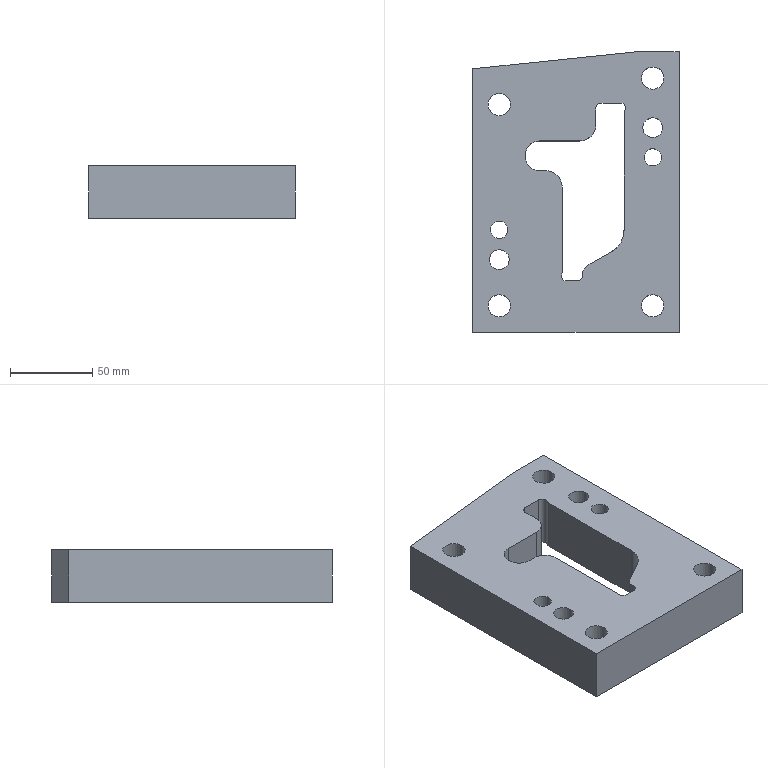Part | STEP file | lll_id230_x_t | 1 solid | 51 faces | box 125 x 170 x 32 mm | volume 507008 mm3 | cylinder 31 | plane 20 | commonest cylinder face diameters 6 x7 13.509 x4 20.008 x4 10.505 x2 12 x2 17.001 x2
STEP:
#1=CARTESIAN_POINT('',(416.145,-122.43,60.5));
#2=VERTEX_POINT('',#1);
#3=CARTESIAN_POINT('',(410.893,-122.43,60.5));
#4=DIRECTION('',(0.,0.,1.));
#5=DIRECTION('',(1.,0.,0.));
#6=AXIS2_PLACEMENT_3D('',#3,#4,#5);
#7=CIRCLE('',#6,5.253);
#8=EDGE_CURVE('',#2,#2,#7,.T.);
#9=ORIENTED_EDGE('',*,*,#8,.T.);
#10=EDGE_LOOP('',(#9));
#11=FACE_BOUND('',#10,.T.);
#12=CARTESIAN_POINT('',(394.893,-24.758,60.5));
#13=VERTEX_POINT('',#12);
#14=CARTESIAN_POINT('',(394.893,-184.43,60.5));
#15=VERTEX_POINT('',#14);
#16=CARTESIAN_POINT('',(394.893,-99.43,60.5));
#17=DIRECTION('',(0.,-1.,0.));
#18=VECTOR('',#17,1.);
#19=LINE('',#16,#18);
#20=EDGE_CURVE('',#13,#15,#19,.T.);
#21=ORIENTED_EDGE('',*,*,#20,.F.);
#22=CARTESIAN_POINT('',(493.966,-14.43,60.5));
#23=VERTEX_POINT('',#22);
#24=CARTESIAN_POINT('',(479.656,-15.922,60.5));
#25=DIRECTION('',(-0.9946,-0.1037,0.));
#26=VECTOR('',#25,1.);
#27=LINE('',#24,#26);
#28=EDGE_CURVE('',#23,#13,#27,.T.);
#29=ORIENTED_EDGE('',*,*,#28,.F.);
#30=CARTESIAN_POINT('',(519.893,-14.43,60.5));
#31=VERTEX_POINT('',#30);
#32=CARTESIAN_POINT('',(457.393,-14.43,60.5));
#33=DIRECTION('',(-1.,0.,0.));
#34=VECTOR('',#33,1.);
#35=LINE('',#32,#34);
#36=EDGE_CURVE('',#31,#23,#35,.T.);
#37=ORIENTED_EDGE('',*,*,#36,.F.);
#38=CARTESIAN_POINT('',(519.893,-184.43,60.5));
#39=VERTEX_POINT('',#38);
#40=CARTESIAN_POINT('',(519.893,-99.43,60.5));
#41=DIRECTION('',(0.,1.,0.));
#42=VECTOR('',#41,1.);
#43=LINE('',#40,#42);
#44=EDGE_CURVE('',#39,#31,#43,.T.);
#45=ORIENTED_EDGE('',*,*,#44,.F.);
#46=CARTESIAN_POINT('',(457.393,-184.43,60.5));
#47=DIRECTION('',(1.,0.,0.));
#48=VECTOR('',#47,1.);
#49=LINE('',#46,#48);
#50=EDGE_CURVE('',#15,#39,#49,.T.);
#51=ORIENTED_EDGE('',*,*,#50,.F.);
#52=EDGE_LOOP('',(#21,#29,#37,#45,#51));
#53=FACE_BOUND('',#52,.T.);
#54=CARTESIAN_POINT('',(416.893,-140.43,60.5));
#55=VERTEX_POINT('',#54);
#56=CARTESIAN_POINT('',(410.893,-140.43,60.5));
#57=DIRECTION('',(0.,0.,-1.));
#58=DIRECTION('',(1.,0.,0.));
#59=AXIS2_PLACEMENT_3D('',#56,#57,#58);
#60=CIRCLE('',#59,6.);
#61=EDGE_CURVE('',#55,#55,#60,.T.);
#62=ORIENTED_EDGE('',*,*,#61,.F.);
#63=EDGE_LOOP('',(#62));
#64=FACE_BOUND('',#63,.T.);
#65=CARTESIAN_POINT('',(509.893,-60.43,60.5));
#66=VERTEX_POINT('',#65);
#67=CARTESIAN_POINT('',(503.893,-60.43,60.5));
#68=DIRECTION('',(0.,0.,-1.));
#69=DIRECTION('',(1.,0.,0.));
#70=AXIS2_PLACEMENT_3D('',#67,#68,#69);
#71=CIRCLE('',#70,6.);
#72=EDGE_CURVE('',#66,#66,#71,.T.);
#73=ORIENTED_EDGE('',*,*,#72,.F.);
#74=EDGE_LOOP('',(#73));
#75=FACE_BOUND('',#74,.T.);
#76=CARTESIAN_POINT('',(400.889,-46.43,60.5));
#77=VERTEX_POINT('',#76);
#78=CARTESIAN_POINT('',(410.893,-46.43,60.5));
#79=DIRECTION('',(0.,0.,1.));
#80=DIRECTION('',(-1.,0.,0.));
#81=AXIS2_PLACEMENT_3D('',#78,#79,#80);
#82=CIRCLE('',#81,10.004);
#83=EDGE_CURVE('',#77,#77,#82,.T.);
#84=ORIENTED_EDGE('',*,*,#83,.T.);
#85=EDGE_LOOP('',(#84));
#86=FACE_BOUND('',#85,.T.);
#87=CARTESIAN_POINT('',(493.889,-30.43,60.5));
#88=VERTEX_POINT('',#87);
#89=CARTESIAN_POINT('',(503.893,-30.43,60.5));
#90=DIRECTION('',(0.,0.,1.));
#91=DIRECTION('',(-1.,0.,0.));
#92=AXIS2_PLACEMENT_3D('',#89,#90,#91);
#93=CIRCLE('',#92,10.004);
#94=EDGE_CURVE('',#88,#88,#93,.T.);
#95=ORIENTED_EDGE('',*,*,#94,.T.);
#96=EDGE_LOOP('',(#95));
#97=FACE_BOUND('',#96,.T.);
#98=CARTESIAN_POINT('',(400.889,-168.43,60.5));
#99=VERTEX_POINT('',#98);
#100=CARTESIAN_POINT('',(410.893,-168.43,60.5));
#101=DIRECTION('',(0.,0.,1.));
#102=DIRECTION('',(-1.,0.,0.));
#103=AXIS2_PLACEMENT_3D('',#100,#101,#102);
#104=CIRCLE('',#103,10.004);
#105=EDGE_CURVE('',#99,#99,#104,.T.);
#106=ORIENTED_EDGE('',*,*,#105,.T.);
#107=EDGE_LOOP('',(#106));
#108=FACE_BOUND('',#107,.T.);
#109=CARTESIAN_POINT('',(493.889,-168.43,60.5));
#110=VERTEX_POINT('',#109);
#111=CARTESIAN_POINT('',(503.893,-168.43,60.5));
#112=DIRECTION('',(0.,0.,1.));
#113=DIRECTION('',(-1.,0.,0.));
#114=AXIS2_PLACEMENT_3D('',#111,#112,#113);
#115=CIRCLE('',#114,10.004);
#116=EDGE_CURVE('',#110,#110,#115,.T.);
#117=ORIENTED_EDGE('',*,*,#116,.T.);
#118=EDGE_LOOP('',(#117));
#119=FACE_BOUND('',#118,.T.);
#120=CARTESIAN_POINT('',(509.145,-78.43,60.5));
#121=VERTEX_POINT('',#120);
#122=CARTESIAN_POINT('',(503.893,-78.43,60.5));
#123=DIRECTION('',(0.,0.,1.));
#124=DIRECTION('',(1.,0.,0.));
#125=AXIS2_PLACEMENT_3D('',#122,#123,#124);
#126=CIRCLE('',#125,5.253);
#127=EDGE_CURVE('',#121,#121,#126,.T.);
#128=ORIENTED_EDGE('',*,*,#127,.T.);
#129=EDGE_LOOP('',(#128));
#130=FACE_BOUND('',#129,.T.);
#131=CARTESIAN_POINT('',(461.369,-147.727,60.5));
#132=VERTEX_POINT('',#131);
#133=CARTESIAN_POINT('',(461.302,-149.551,60.5));
#134=VERTEX_POINT('',#133);
#135=CARTESIAN_POINT('',(464.191,-148.744,60.5));
#136=DIRECTION('',(0.,0.,1.));
#137=DIRECTION('',(-1.,0.,0.));
#138=AXIS2_PLACEMENT_3D('',#135,#136,#137);
#139=CIRCLE('',#138,3.);
#140=EDGE_CURVE('',#132,#134,#139,.T.);
#141=ORIENTED_EDGE('',*,*,#140,.F.);
#142=CARTESIAN_POINT('',(465.269,-143.286,60.5));
#143=VERTEX_POINT('',#142);
#144=CARTESIAN_POINT('',(468.962,-150.461,60.5));
#145=DIRECTION('',(0.,0.,-1.));
#146=DIRECTION('',(-1.,0.,0.));
#147=AXIS2_PLACEMENT_3D('',#144,#145,#146);
#148=CIRCLE('',#147,8.07);
#149=EDGE_CURVE('',#132,#143,#148,.T.);
#150=ORIENTED_EDGE('',*,*,#149,.T.);
#151=CARTESIAN_POINT('',(478.829,-135.663,60.5));
#152=VERTEX_POINT('',#151);
#153=CARTESIAN_POINT('',(478.018,-136.119,60.5));
#154=DIRECTION('',(-0.8717,-0.49,0.));
#155=VECTOR('',#154,1.);
#156=LINE('',#153,#155);
#157=EDGE_CURVE('',#152,#143,#156,.T.);
#158=ORIENTED_EDGE('',*,*,#157,.F.);
#159=CARTESIAN_POINT('',(479.654,-135.117,60.5));
#160=VERTEX_POINT('',#159);
#161=CARTESIAN_POINT('',(448.181,-88.407,60.5));
#162=DIRECTION('',(0.,0.,-1.));
#163=DIRECTION('',(-1.,0.,0.));
#164=AXIS2_PLACEMENT_3D('',#161,#162,#163);
#165=CIRCLE('',#164,56.324);
#166=EDGE_CURVE('',#160,#152,#165,.T.);
#167=ORIENTED_EDGE('',*,*,#166,.F.);
#168=CARTESIAN_POINT('',(480.466,-134.556,60.5));
#169=VERTEX_POINT('',#168);
#170=CARTESIAN_POINT('',(462.354,-109.242,60.5));
#171=DIRECTION('',(0.,0.,-1.));
#172=DIRECTION('',(-1.,0.,0.));
#173=AXIS2_PLACEMENT_3D('',#170,#171,#172);
#174=CIRCLE('',#173,31.126);
#175=EDGE_CURVE('',#169,#160,#174,.T.);
#176=ORIENTED_EDGE('',*,*,#175,.F.);
#177=CARTESIAN_POINT('',(481.25,-133.962,60.5));
#178=VERTEX_POINT('',#177);
#179=CARTESIAN_POINT('',(469.718,-119.534,60.5));
#180=DIRECTION('',(0.,0.,1.));
#181=DIRECTION('',(-1.,0.,0.));
#182=AXIS2_PLACEMENT_3D('',#179,#180,#181);
#183=CIRCLE('',#182,18.471);
#184=EDGE_CURVE('',#169,#178,#183,.T.);
#185=ORIENTED_EDGE('',*,*,#184,.T.);
#186=CARTESIAN_POINT('',(482.171,-133.152,60.5));
#187=VERTEX_POINT('',#186);
#188=CARTESIAN_POINT('',(473.427,-124.145,60.5));
#189=DIRECTION('',(0.,0.,1.));
#190=DIRECTION('',(-1.,0.,0.));
#191=AXIS2_PLACEMENT_3D('',#188,#189,#190);
#192=CIRCLE('',#191,12.553);
#193=EDGE_CURVE('',#178,#187,#192,.T.);
#194=ORIENTED_EDGE('',*,*,#193,.T.);
#195=CARTESIAN_POINT('',(484.678,-129.804,60.5));
#196=VERTEX_POINT('',#195);
#197=CARTESIAN_POINT('',(472.01,-122.929,60.5));
#198=DIRECTION('',(0.,0.,1.));
#199=DIRECTION('',(-1.,0.,0.));
#200=AXIS2_PLACEMENT_3D('',#197,#198,#199);
#201=CIRCLE('',#200,14.414);
#202=EDGE_CURVE('',#187,#196,#201,.T.);
#203=ORIENTED_EDGE('',*,*,#202,.T.);
#204=CARTESIAN_POINT('',(486.461,-123.716,60.5));
#205=VERTEX_POINT('',#204);
#206=CARTESIAN_POINT('',(472.347,-122.889,60.5));
#207=DIRECTION('',(0.,0.,-1.));
#208=DIRECTION('',(-1.,0.,0.));
#209=AXIS2_PLACEMENT_3D('',#206,#207,#208);
#210=CIRCLE('',#209,14.138);
#211=EDGE_CURVE('',#205,#196,#210,.T.);
#212=ORIENTED_EDGE('',*,*,#211,.F.);
#213=CARTESIAN_POINT('',(486.506,-122.731,60.5));
#214=VERTEX_POINT('',#213);
#215=CARTESIAN_POINT('',(439.156,-121.059,60.5));
#216=DIRECTION('',(0.,0.,-1.));
#217=DIRECTION('',(-1.,0.,0.));
#218=AXIS2_PLACEMENT_3D('',#215,#216,#217);
#219=CIRCLE('',#218,47.38);
#220=EDGE_CURVE('',#214,#205,#219,.T.);
#221=ORIENTED_EDGE('',*,*,#220,.F.);
#222=CARTESIAN_POINT('',(486.51,-51.898,60.5));
#223=VERTEX_POINT('',#222);
#224=CARTESIAN_POINT('',(486.507,-99.431,60.5));
#225=DIRECTION('',(0.00006142,1.,0.));
#226=VECTOR('',#225,1.);
#227=LINE('',#224,#226);
#228=EDGE_CURVE('',#214,#223,#227,.T.);
#229=ORIENTED_EDGE('',*,*,#228,.T.);
#230=CARTESIAN_POINT('',(487.038,-50.199,60.5));
#231=VERTEX_POINT('',#230);
#232=CARTESIAN_POINT('',(489.51,-51.898,60.5));
#233=DIRECTION('',(0.,0.,1.));
#234=DIRECTION('',(-1.,0.,0.));
#235=AXIS2_PLACEMENT_3D('',#232,#233,#234);
#236=CIRCLE('',#235,3.);
#237=EDGE_CURVE('',#231,#223,#236,.T.);
#238=ORIENTED_EDGE('',*,*,#237,.F.);
#239=CARTESIAN_POINT('',(484.565,-45.5,60.5));
#240=VERTEX_POINT('',#239);
#241=CARTESIAN_POINT('',(484.565,-48.5,60.5));
#242=DIRECTION('',(0.,0.,-1.));
#243=DIRECTION('',(-1.,0.,0.));
#244=AXIS2_PLACEMENT_3D('',#241,#242,#243);
#245=CIRCLE('',#244,3.);
#246=EDGE_CURVE('',#240,#231,#245,.T.);
#247=ORIENTED_EDGE('',*,*,#246,.F.);
#248=CARTESIAN_POINT('',(472.5,-45.5,60.5));
#249=VERTEX_POINT('',#248);
#250=CARTESIAN_POINT('',(457.393,-45.5,60.5));
#251=DIRECTION('',(-1.,0.,0.));
#252=VECTOR('',#251,1.);
#253=LINE('',#250,#252);
#254=EDGE_CURVE('',#240,#249,#253,.T.);
#255=ORIENTED_EDGE('',*,*,#254,.T.);
#256=CARTESIAN_POINT('',(469.5,-48.5,60.5));
#257=VERTEX_POINT('',#256);
#258=CARTESIAN_POINT('',(472.5,-48.5,60.5));
#259=DIRECTION('',(0.,0.,1.));
#260=DIRECTION('',(-1.,0.,0.));
#261=AXIS2_PLACEMENT_3D('',#258,#259,#260);
#262=CIRCLE('',#261,3.);
#263=EDGE_CURVE('',#249,#257,#262,.T.);
#264=ORIENTED_EDGE('',*,*,#263,.T.);
#265=CARTESIAN_POINT('',(469.5,-58.5,60.5));
#266=VERTEX_POINT('',#265);
#267=CARTESIAN_POINT('',(469.5,-99.43,60.5));
#268=DIRECTION('',(0.,1.,0.));
#269=VECTOR('',#268,1.);
#270=LINE('',#267,#269);
#271=EDGE_CURVE('',#266,#257,#270,.T.);
#272=ORIENTED_EDGE('',*,*,#271,.F.);
#273=CARTESIAN_POINT('',(459.5,-68.5,60.5));
#274=VERTEX_POINT('',#273);
#275=CARTESIAN_POINT('',(459.499,-58.499,60.5));
#276=DIRECTION('',(0.,0.,1.));
#277=DIRECTION('',(-1.,0.,0.));
#278=AXIS2_PLACEMENT_3D('',#275,#276,#277);
#279=CIRCLE('',#278,10.001);
#280=EDGE_CURVE('',#274,#266,#279,.T.);
#281=ORIENTED_EDGE('',*,*,#280,.F.);
#282=CARTESIAN_POINT('',(435.2,-68.5,60.5));
#283=VERTEX_POINT('',#282);
#284=CARTESIAN_POINT('',(457.393,-68.5,60.5));
#285=DIRECTION('',(1.,0.,0.));
#286=VECTOR('',#285,1.);
#287=LINE('',#284,#286);
#288=EDGE_CURVE('',#283,#274,#287,.T.);
#289=ORIENTED_EDGE('',*,*,#288,.F.);
#290=CARTESIAN_POINT('',(426.7,-77.,60.5));
#291=VERTEX_POINT('',#290);
#292=CARTESIAN_POINT('',(435.2,-77.,60.5));
#293=DIRECTION('',(0.,0.,1.));
#294=DIRECTION('',(-1.,0.,0.));
#295=AXIS2_PLACEMENT_3D('',#292,#293,#294);
#296=CIRCLE('',#295,8.5);
#297=EDGE_CURVE('',#283,#291,#296,.T.);
#298=ORIENTED_EDGE('',*,*,#297,.T.);
#299=CARTESIAN_POINT('',(426.7,-78.,60.5));
#300=VERTEX_POINT('',#299);
#301=CARTESIAN_POINT('',(426.7,-99.43,60.5));
#302=DIRECTION('',(0.,1.,0.));
#303=VECTOR('',#302,1.);
#304=LINE('',#301,#303);
#305=EDGE_CURVE('',#300,#291,#304,.T.);
#306=ORIENTED_EDGE('',*,*,#305,.F.);
#307=CARTESIAN_POINT('',(435.2,-86.5,60.5));
#308=VERTEX_POINT('',#307);
#309=CARTESIAN_POINT('',(435.2,-78.,60.5));
#310=DIRECTION('',(0.,0.,1.));
#311=DIRECTION('',(-1.,0.,0.));
#312=AXIS2_PLACEMENT_3D('',#309,#310,#311);
#313=CIRCLE('',#312,8.5);
#314=EDGE_CURVE('',#300,#308,#313,.T.);
#315=ORIENTED_EDGE('',*,*,#314,.T.);
#316=CARTESIAN_POINT('',(439.,-86.5,60.5));
#317=VERTEX_POINT('',#316);
#318=CARTESIAN_POINT('',(457.393,-86.5,60.5));
#319=DIRECTION('',(-1.,0.,0.));
#320=VECTOR('',#319,1.);
#321=LINE('',#318,#320);
#322=EDGE_CURVE('',#317,#308,#321,.T.);
#323=ORIENTED_EDGE('',*,*,#322,.F.);
#324=CARTESIAN_POINT('',(449.,-96.5,60.5));
#325=VERTEX_POINT('',#324);
#326=CARTESIAN_POINT('',(438.999,-96.501,60.5));
#327=DIRECTION('',(0.,0.,1.));
#328=DIRECTION('',(-1.,0.,0.));
#329=AXIS2_PLACEMENT_3D('',#326,#327,#328);
#330=CIRCLE('',#329,10.001);
#331=EDGE_CURVE('',#325,#317,#330,.T.);
#332=ORIENTED_EDGE('',*,*,#331,.F.);
#333=CARTESIAN_POINT('',(449.,-147.961,60.5));
#334=VERTEX_POINT('',#333);
#335=CARTESIAN_POINT('',(449.,-99.43,60.5));
#336=DIRECTION('',(0.,-1.,0.));
#337=VECTOR('',#336,1.);
#338=LINE('',#335,#337);
#339=EDGE_CURVE('',#325,#334,#338,.T.);
#340=ORIENTED_EDGE('',*,*,#339,.T.);
#341=CARTESIAN_POINT('',(448.75,-149.16,60.5));
#342=VERTEX_POINT('',#341);
#343=CARTESIAN_POINT('',(446.,-147.961,60.5));
#344=DIRECTION('',(0.,0.,-1.));
#345=DIRECTION('',(-1.,0.,0.));
#346=AXIS2_PLACEMENT_3D('',#343,#344,#345);
#347=CIRCLE('',#346,3.);
#348=EDGE_CURVE('',#334,#342,#347,.T.);
#349=ORIENTED_EDGE('',*,*,#348,.T.);
#350=CARTESIAN_POINT('',(451.5,-153.359,60.5));
#351=VERTEX_POINT('',#350);
#352=CARTESIAN_POINT('',(451.5,-150.359,60.5));
#353=DIRECTION('',(0.,0.,1.));
#354=DIRECTION('',(-1.,0.,0.));
#355=AXIS2_PLACEMENT_3D('',#352,#353,#354);
#356=CIRCLE('',#355,3.);
#357=EDGE_CURVE('',#342,#351,#356,.T.);
#358=ORIENTED_EDGE('',*,*,#357,.T.);
#359=CARTESIAN_POINT('',(458.413,-153.359,60.5));
#360=VERTEX_POINT('',#359);
#361=CARTESIAN_POINT('',(457.393,-153.359,60.5));
#362=DIRECTION('',(-1.,0.,0.));
#363=VECTOR('',#362,1.);
#364=LINE('',#361,#363);
#365=EDGE_CURVE('',#360,#351,#364,.T.);
#366=ORIENTED_EDGE('',*,*,#365,.F.);
#367=CARTESIAN_POINT('',(458.413,-150.359,60.5));
#368=DIRECTION('',(0.,0.,1.));
#369=DIRECTION('',(-1.,0.,0.));
#370=AXIS2_PLACEMENT_3D('',#367,#368,#369);
#371=CIRCLE('',#370,3.);
#372=EDGE_CURVE('',#360,#134,#371,.T.);
#373=ORIENTED_EDGE('',*,*,#372,.T.);
#374=EDGE_LOOP('',(#141,#150,#158,#167,#176,#185,#194,#203,#212,#221,#229,#238,#247,#255,#264,#272,#281,#289,#298,#306,#315,#323,#332,#340,#349,#358,#366,#373));
#375=FACE_BOUND('',#374,.T.);
#376=CARTESIAN_POINT('',(457.393,-99.43,60.5));
#377=DIRECTION('',(0.,0.,-1.));
#378=DIRECTION('',(1.,0.,0.));
#379=AXIS2_PLACEMENT_3D('',#376,#377,#378);
#380=PLANE('',#379);
#381=ADVANCED_FACE('',(#11,#53,#64,#75,#86,#97,#108,#119,#130,#375),#380,.T.);
#382=CARTESIAN_POINT('',(497.138,-30.43,92.5));
#383=VERTEX_POINT('',#382);
#384=CARTESIAN_POINT('',(503.893,-30.43,92.5));
#385=DIRECTION('',(0.,0.,1.));
#386=DIRECTION('',(-1.,0.,0.));
#387=AXIS2_PLACEMENT_3D('',#384,#385,#386);
#388=CIRCLE('',#387,6.755);
#389=EDGE_CURVE('',#383,#383,#388,.T.);
#390=ORIENTED_EDGE('',*,*,#389,.F.);
#391=EDGE_LOOP('',(#390));
#392=FACE_BOUND('',#391,.T.);
#393=CARTESIAN_POINT('',(404.138,-168.43,92.5));
#394=VERTEX_POINT('',#393);
#395=CARTESIAN_POINT('',(410.893,-168.43,92.5));
#396=DIRECTION('',(0.,0.,1.));
#397=DIRECTION('',(-1.,0.,0.));
#398=AXIS2_PLACEMENT_3D('',#395,#396,#397);
#399=CIRCLE('',#398,6.755);
#400=EDGE_CURVE('',#394,#394,#399,.T.);
#401=ORIENTED_EDGE('',*,*,#400,.F.);
#402=EDGE_LOOP('',(#401));
#403=FACE_BOUND('',#402,.T.);
#404=CARTESIAN_POINT('',(404.138,-46.43,92.5));
#405=VERTEX_POINT('',#404);
#406=CARTESIAN_POINT('',(410.893,-46.43,92.5));
#407=DIRECTION('',(0.,0.,1.));
#408=DIRECTION('',(-1.,0.,0.));
#409=AXIS2_PLACEMENT_3D('',#406,#407,#408);
#410=CIRCLE('',#409,6.755);
#411=EDGE_CURVE('',#405,#405,#410,.T.);
#412=ORIENTED_EDGE('',*,*,#411,.F.);
#413=EDGE_LOOP('',(#412));
#414=FACE_BOUND('',#413,.T.);
#415=CARTESIAN_POINT('',(497.138,-168.43,92.5));
#416=VERTEX_POINT('',#415);
#417=CARTESIAN_POINT('',(503.893,-168.43,92.5));
#418=DIRECTION('',(0.,0.,1.));
#419=DIRECTION('',(-1.,0.,0.));
#420=AXIS2_PLACEMENT_3D('',#417,#418,#419);
#421=CIRCLE('',#420,6.755);
#422=EDGE_CURVE('',#416,#416,#421,.T.);
#423=ORIENTED_EDGE('',*,*,#422,.F.);
#424=EDGE_LOOP('',(#423));
#425=FACE_BOUND('',#424,.T.);
#426=CARTESIAN_POINT('',(497.893,-60.43,92.5));
#427=VERTEX_POINT('',#426);
#428=CARTESIAN_POINT('',(503.893,-60.43,92.5));
#429=DIRECTION('',(0.,0.,1.));
#430=DIRECTION('',(-1.,0.,0.));
#431=AXIS2_PLACEMENT_3D('',#428,#429,#430);
#432=CIRCLE('',#431,6.);
#433=EDGE_CURVE('',#427,#427,#432,.T.);
#434=ORIENTED_EDGE('',*,*,#433,.F.);
#435=EDGE_LOOP('',(#434));
#436=FACE_BOUND('',#435,.T.);
#437=CARTESIAN_POINT('',(404.893,-140.43,92.5));
#438=VERTEX_POINT('',#437);
#439=CARTESIAN_POINT('',(410.893,-140.43,92.5));
#440=DIRECTION('',(0.,0.,1.));
#441=DIRECTION('',(-1.,0.,0.));
#442=AXIS2_PLACEMENT_3D('',#439,#440,#441);
#443=CIRCLE('',#442,6.);
#444=EDGE_CURVE('',#438,#438,#443,.T.);
#445=ORIENTED_EDGE('',*,*,#444,.F.);
#446=EDGE_LOOP('',(#445));
#447=FACE_BOUND('',#446,.T.);
#448=CARTESIAN_POINT('',(493.966,-14.43,92.5));
#449=VERTEX_POINT('',#448);
#450=CARTESIAN_POINT('',(519.893,-14.43,92.5));
#451=VERTEX_POINT('',#450);
#452=CARTESIAN_POINT('',(457.393,-14.43,92.5));
#453=DIRECTION('',(1.,0.,0.));
#454=VECTOR('',#453,1.);
#455=LINE('',#452,#454);
#456=EDGE_CURVE('',#449,#451,#455,.T.);
#457=ORIENTED_EDGE('',*,*,#456,.F.);
#458=CARTESIAN_POINT('',(394.893,-24.758,92.5));
#459=VERTEX_POINT('',#458);
#460=CARTESIAN_POINT('',(479.656,-15.922,92.5));
#461=DIRECTION('',(0.9946,0.1037,0.));
#462=VECTOR('',#461,1.);
#463=LINE('',#460,#462);
#464=EDGE_CURVE('',#459,#449,#463,.T.);
#465=ORIENTED_EDGE('',*,*,#464,.F.);
#466=CARTESIAN_POINT('',(394.893,-184.43,92.5));
#467=VERTEX_POINT('',#466);
#468=CARTESIAN_POINT('',(394.893,-99.43,92.5));
#469=DIRECTION('',(0.,1.,0.));
#470=VECTOR('',#469,1.);
#471=LINE('',#468,#470);
#472=EDGE_CURVE('',#467,#459,#471,.T.);
#473=ORIENTED_EDGE('',*,*,#472,.F.);
#474=CARTESIAN_POINT('',(519.893,-184.43,92.5));
#475=VERTEX_POINT('',#474);
#476=CARTESIAN_POINT('',(457.393,-184.43,92.5));
#477=DIRECTION('',(-1.,0.,0.));
#478=VECTOR('',#477,1.);
#479=LINE('',#476,#478);
#480=EDGE_CURVE('',#475,#467,#479,.T.);
#481=ORIENTED_EDGE('',*,*,#480,.F.);
#482=CARTESIAN_POINT('',(519.893,-99.43,92.5));
#483=DIRECTION('',(0.,-1.,0.));
#484=VECTOR('',#483,1.);
#485=LINE('',#482,#484);
#486=EDGE_CURVE('',#451,#475,#485,.T.);
#487=ORIENTED_EDGE('',*,*,#486,.F.);
#488=EDGE_LOOP('',(#457,#465,#473,#481,#487));
#489=FACE_BOUND('',#488,.T.);
#490=CARTESIAN_POINT('',(509.145,-78.43,92.5));
#491=VERTEX_POINT('',#490);
#492=CARTESIAN_POINT('',(503.893,-78.43,92.5));
#493=DIRECTION('',(0.,0.,1.));
#494=DIRECTION('',(1.,0.,0.));
#495=AXIS2_PLACEMENT_3D('',#492,#493,#494);
#496=CIRCLE('',#495,5.253);
#497=EDGE_CURVE('',#491,#491,#496,.T.);
#498=ORIENTED_EDGE('',*,*,#497,.F.);
#499=EDGE_LOOP('',(#498));
#500=FACE_BOUND('',#499,.T.);
#501=CARTESIAN_POINT('',(416.145,-122.43,92.5));
#502=VERTEX_POINT('',#501);
#503=CARTESIAN_POINT('',(410.893,-122.43,92.5));
#504=DIRECTION('',(0.,0.,1.));
#505=DIRECTION('',(1.,0.,0.));
#506=AXIS2_PLACEMENT_3D('',#503,#504,#505);
#507=CIRCLE('',#506,5.253);
#508=EDGE_CURVE('',#502,#502,#507,.T.);
#509=ORIENTED_EDGE('',*,*,#508,.F.);
#510=EDGE_LOOP('',(#509));
#511=FACE_BOUND('',#510,.T.);
#512=CARTESIAN_POINT('',(465.269,-143.286,92.5));
#513=VERTEX_POINT('',#512);
#514=CARTESIAN_POINT('',(478.829,-135.663,92.5));
#515=VERTEX_POINT('',#514);
#516=CARTESIAN_POINT('',(478.018,-136.119,92.5));
#517=DIRECTION('',(0.8717,0.49,0.));
#518=VECTOR('',#517,1.);
#519=LINE('',#516,#518);
#520=EDGE_CURVE('',#513,#515,#519,.T.);
#521=ORIENTED_EDGE('',*,*,#520,.F.);
#522=CARTESIAN_POINT('',(461.369,-147.727,92.5));
#523=VERTEX_POINT('',#522);
#524=CARTESIAN_POINT('',(468.962,-150.461,92.5));
#525=DIRECTION('',(0.,0.,1.));
#526=DIRECTION('',(1.,0.,0.));
#527=AXIS2_PLACEMENT_3D('',#524,#525,#526);
#528=CIRCLE('',#527,8.07);
#529=EDGE_CURVE('',#513,#523,#528,.T.);
#530=ORIENTED_EDGE('',*,*,#529,.T.);
#531=CARTESIAN_POINT('',(461.302,-149.551,92.5));
#532=VERTEX_POINT('',#531);
#533=CARTESIAN_POINT('',(464.191,-148.744,92.5));
#534=DIRECTION('',(0.,0.,-1.));
#535=DIRECTION('',(1.,0.,0.));
#536=AXIS2_PLACEMENT_3D('',#533,#534,#535);
#537=CIRCLE('',#536,3.);
#538=EDGE_CURVE('',#532,#523,#537,.T.);
#539=ORIENTED_EDGE('',*,*,#538,.F.);
#540=CARTESIAN_POINT('',(458.413,-153.359,92.5));
#541=VERTEX_POINT('',#540);
#542=CARTESIAN_POINT('',(458.413,-150.359,92.5));
#543=DIRECTION('',(0.,0.,-1.));
#544=DIRECTION('',(1.,0.,0.));
#545=AXIS2_PLACEMENT_3D('',#542,#543,#544);
#546=CIRCLE('',#545,3.);
#547=EDGE_CURVE('',#532,#541,#546,.T.);
#548=ORIENTED_EDGE('',*,*,#547,.T.);
#549=CARTESIAN_POINT('',(451.5,-153.359,92.5));
#550=VERTEX_POINT('',#549);
#551=CARTESIAN_POINT('',(457.393,-153.359,92.5));
#552=DIRECTION('',(1.,0.,0.));
#553=VECTOR('',#552,1.);
#554=LINE('',#551,#553);
#555=EDGE_CURVE('',#550,#541,#554,.T.);
#556=ORIENTED_EDGE('',*,*,#555,.F.);
#557=CARTESIAN_POINT('',(448.75,-149.16,92.5));
#558=VERTEX_POINT('',#557);
#559=CARTESIAN_POINT('',(451.5,-150.359,92.5));
#560=DIRECTION('',(0.,0.,-1.));
#561=DIRECTION('',(1.,0.,0.));
#562=AXIS2_PLACEMENT_3D('',#559,#560,#561);
#563=CIRCLE('',#562,3.);
#564=EDGE_CURVE('',#550,#558,#563,.T.);
#565=ORIENTED_EDGE('',*,*,#564,.T.);
#566=CARTESIAN_POINT('',(449.,-147.961,92.5));
#567=VERTEX_POINT('',#566);
#568=CARTESIAN_POINT('',(446.,-147.961,92.5));
#569=DIRECTION('',(0.,0.,-1.));
#570=DIRECTION('',(1.,0.,0.));
#571=AXIS2_PLACEMENT_3D('',#568,#569,#570);
#572=CIRCLE('',#571,3.);
#573=EDGE_CURVE('',#567,#558,#572,.T.);
#574=ORIENTED_EDGE('',*,*,#573,.F.);
#575=CARTESIAN_POINT('',(449.,-96.5,92.5));
#576=VERTEX_POINT('',#575);
#577=CARTESIAN_POINT('',(449.,-99.43,92.5));
#578=DIRECTION('',(0.,1.,0.));
#579=VECTOR('',#578,1.);
#580=LINE('',#577,#579);
#581=EDGE_CURVE('',#567,#576,#580,.T.);
#582=ORIENTED_EDGE('',*,*,#581,.T.);
#583=CARTESIAN_POINT('',(439.,-86.5,92.5));
#584=VERTEX_POINT('',#583);
#585=CARTESIAN_POINT('',(438.999,-96.501,92.5));
#586=DIRECTION('',(0.,0.,-1.));
#587=DIRECTION('',(1.,0.,0.));
#588=AXIS2_PLACEMENT_3D('',#585,#586,#587);
#589=CIRCLE('',#588,10.001);
#590=EDGE_CURVE('',#584,#576,#589,.T.);
#591=ORIENTED_EDGE('',*,*,#590,.F.);
#592=CARTESIAN_POINT('',(435.2,-86.5,92.5));
#593=VERTEX_POINT('',#592);
#594=CARTESIAN_POINT('',(457.393,-86.5,92.5));
#595=DIRECTION('',(1.,0.,0.));
#596=VECTOR('',#595,1.);
#597=LINE('',#594,#596);
#598=EDGE_CURVE('',#593,#584,#597,.T.);
#599=ORIENTED_EDGE('',*,*,#598,.F.);
#600=CARTESIAN_POINT('',(426.7,-78.,92.5));
#601=VERTEX_POINT('',#600);
#602=CARTESIAN_POINT('',(435.2,-78.,92.5));
#603=DIRECTION('',(0.,0.,-1.));
#604=DIRECTION('',(1.,0.,0.));
#605=AXIS2_PLACEMENT_3D('',#602,#603,#604);
#606=CIRCLE('',#605,8.5);
#607=EDGE_CURVE('',#593,#601,#606,.T.);
#608=ORIENTED_EDGE('',*,*,#607,.T.);
#609=CARTESIAN_POINT('',(426.7,-77.,92.5));
#610=VERTEX_POINT('',#609);
#611=CARTESIAN_POINT('',(426.7,-99.43,92.5));
#612=DIRECTION('',(0.,-1.,0.));
#613=VECTOR('',#612,1.);
#614=LINE('',#611,#613);
#615=EDGE_CURVE('',#610,#601,#614,.T.);
#616=ORIENTED_EDGE('',*,*,#615,.F.);
#617=CARTESIAN_POINT('',(435.2,-68.5,92.5));
#618=VERTEX_POINT('',#617);
#619=CARTESIAN_POINT('',(435.2,-77.,92.5));
#620=DIRECTION('',(0.,0.,-1.));
#621=DIRECTION('',(1.,0.,0.));
#622=AXIS2_PLACEMENT_3D('',#619,#620,#621);
#623=CIRCLE('',#622,8.5);
#624=EDGE_CURVE('',#610,#618,#623,.T.);
#625=ORIENTED_EDGE('',*,*,#624,.T.);
#626=CARTESIAN_POINT('',(459.5,-68.5,92.5));
#627=VERTEX_POINT('',#626);
#628=CARTESIAN_POINT('',(457.393,-68.5,92.5));
#629=DIRECTION('',(-1.,0.,0.));
#630=VECTOR('',#629,1.);
#631=LINE('',#628,#630);
#632=EDGE_CURVE('',#627,#618,#631,.T.);
#633=ORIENTED_EDGE('',*,*,#632,.F.);
#634=CARTESIAN_POINT('',(469.5,-58.5,92.5));
#635=VERTEX_POINT('',#634);
#636=CARTESIAN_POINT('',(459.499,-58.499,92.5));
#637=DIRECTION('',(0.,0.,1.));
#638=DIRECTION('',(1.,0.,0.));
#639=AXIS2_PLACEMENT_3D('',#636,#637,#638);
#640=CIRCLE('',#639,10.001);
#641=EDGE_CURVE('',#627,#635,#640,.T.);
#642=ORIENTED_EDGE('',*,*,#641,.T.);
#643=CARTESIAN_POINT('',(469.5,-48.5,92.5));
#644=VERTEX_POINT('',#643);
#645=CARTESIAN_POINT('',(469.5,-99.43,92.5));
#646=DIRECTION('',(0.,1.,0.));
#647=VECTOR('',#646,1.);
#648=LINE('',#645,#647);
#649=EDGE_CURVE('',#635,#644,#648,.T.);
#650=ORIENTED_EDGE('',*,*,#649,.T.);
#651=CARTESIAN_POINT('',(472.5,-45.5,92.5));
#652=VERTEX_POINT('',#651);
#653=CARTESIAN_POINT('',(472.5,-48.5,92.5));
#654=DIRECTION('',(0.,0.,1.));
#655=DIRECTION('',(1.,0.,0.));
#656=AXIS2_PLACEMENT_3D('',#653,#654,#655);
#657=CIRCLE('',#656,3.);
#658=EDGE_CURVE('',#652,#644,#657,.T.);
#659=ORIENTED_EDGE('',*,*,#658,.F.);
#660=CARTESIAN_POINT('',(484.565,-45.5,92.5));
#661=VERTEX_POINT('',#660);
#662=CARTESIAN_POINT('',(457.393,-45.5,92.5));
#663=DIRECTION('',(1.,0.,0.));
#664=VECTOR('',#663,1.);
#665=LINE('',#662,#664);
#666=EDGE_CURVE('',#652,#661,#665,.T.);
#667=ORIENTED_EDGE('',*,*,#666,.T.);
#668=CARTESIAN_POINT('',(487.038,-50.199,92.5));
#669=VERTEX_POINT('',#668);
#670=CARTESIAN_POINT('',(484.565,-48.5,92.5));
#671=DIRECTION('',(0.,0.,1.));
#672=DIRECTION('',(1.,0.,0.));
#673=AXIS2_PLACEMENT_3D('',#670,#671,#672);
#674=CIRCLE('',#673,3.);
#675=EDGE_CURVE('',#669,#661,#674,.T.);
#676=ORIENTED_EDGE('',*,*,#675,.F.);
#677=CARTESIAN_POINT('',(486.51,-51.898,92.5));
#678=VERTEX_POINT('',#677);
#679=CARTESIAN_POINT('',(489.51,-51.898,92.5));
#680=DIRECTION('',(0.,0.,-1.));
#681=DIRECTION('',(1.,0.,0.));
#682=AXIS2_PLACEMENT_3D('',#679,#680,#681);
#683=CIRCLE('',#682,3.);
#684=EDGE_CURVE('',#678,#669,#683,.T.);
#685=ORIENTED_EDGE('',*,*,#684,.F.);
#686=CARTESIAN_POINT('',(486.506,-122.731,92.5));
#687=VERTEX_POINT('',#686);
#688=CARTESIAN_POINT('',(486.507,-99.431,92.5));
#689=DIRECTION('',(0.00006142,1.,0.));
#690=VECTOR('',#689,1.);
#691=LINE('',#688,#690);
#692=EDGE_CURVE('',#687,#678,#691,.T.);
#693=ORIENTED_EDGE('',*,*,#692,.F.);
#694=CARTESIAN_POINT('',(486.461,-123.716,92.5));
#695=VERTEX_POINT('',#694);
#696=CARTESIAN_POINT('',(439.156,-121.059,92.5));
#697=DIRECTION('',(0.,0.,-1.));
#698=DIRECTION('',(1.,0.,0.));
#699=AXIS2_PLACEMENT_3D('',#696,#697,#698);
#700=CIRCLE('',#699,47.38);
#701=EDGE_CURVE('',#687,#695,#700,.T.);
#702=ORIENTED_EDGE('',*,*,#701,.T.);
#703=CARTESIAN_POINT('',(484.678,-129.804,92.5));
#704=VERTEX_POINT('',#703);
#705=CARTESIAN_POINT('',(472.347,-122.889,92.5));
#706=DIRECTION('',(0.,0.,-1.));
#707=DIRECTION('',(1.,0.,0.));
#708=AXIS2_PLACEMENT_3D('',#705,#706,#707);
#709=CIRCLE('',#708,14.138);
#710=EDGE_CURVE('',#695,#704,#709,.T.);
#711=ORIENTED_EDGE('',*,*,#710,.T.);
#712=CARTESIAN_POINT('',(482.171,-133.152,92.5));
#713=VERTEX_POINT('',#712);
#714=CARTESIAN_POINT('',(472.01,-122.929,92.5));
#715=DIRECTION('',(0.,0.,1.));
#716=DIRECTION('',(1.,0.,0.));
#717=AXIS2_PLACEMENT_3D('',#714,#715,#716);
#718=CIRCLE('',#717,14.414);
#719=EDGE_CURVE('',#713,#704,#718,.T.);
#720=ORIENTED_EDGE('',*,*,#719,.F.);
#721=CARTESIAN_POINT('',(481.25,-133.962,92.5));
#722=VERTEX_POINT('',#721);
#723=CARTESIAN_POINT('',(473.427,-124.145,92.5));
#724=DIRECTION('',(0.,0.,1.));
#725=DIRECTION('',(1.,0.,0.));
#726=AXIS2_PLACEMENT_3D('',#723,#724,#725);
#727=CIRCLE('',#726,12.553);
#728=EDGE_CURVE('',#722,#713,#727,.T.);
#729=ORIENTED_EDGE('',*,*,#728,.F.);
#730=CARTESIAN_POINT('',(480.466,-134.556,92.5));
#731=VERTEX_POINT('',#730);
#732=CARTESIAN_POINT('',(469.718,-119.534,92.5));
#733=DIRECTION('',(0.,0.,-1.));
#734=DIRECTION('',(1.,0.,0.));
#735=AXIS2_PLACEMENT_3D('',#732,#733,#734);
#736=CIRCLE('',#735,18.471);
#737=EDGE_CURVE('',#722,#731,#736,.T.);
#738=ORIENTED_EDGE('',*,*,#737,.T.);
#739=CARTESIAN_POINT('',(479.654,-135.117,92.5));
#740=VERTEX_POINT('',#739);
#741=CARTESIAN_POINT('',(462.354,-109.242,92.5));
#742=DIRECTION('',(0.,0.,-1.));
#743=DIRECTION('',(1.,0.,0.));
#744=AXIS2_PLACEMENT_3D('',#741,#742,#743);
#745=CIRCLE('',#744,31.126);
#746=EDGE_CURVE('',#731,#740,#745,.T.);
#747=ORIENTED_EDGE('',*,*,#746,.T.);
#748=CARTESIAN_POINT('',(448.181,-88.407,92.5));
#749=DIRECTION('',(0.,0.,1.));
#750=DIRECTION('',(1.,0.,0.));
#751=AXIS2_PLACEMENT_3D('',#748,#749,#750);
#752=CIRCLE('',#751,56.324);
#753=EDGE_CURVE('',#515,#740,#752,.T.);
#754=ORIENTED_EDGE('',*,*,#753,.F.);
#755=EDGE_LOOP('',(#521,#530,#539,#548,#556,#565,#574,#582,#591,#599,#608,#616,#625,#633,#642,#650,#659,#667,#676,#685,#693,#702,#711,#720,#729,#738,#747,#754));
#756=FACE_BOUND('',#755,.T.);
#757=CARTESIAN_POINT('',(457.393,-99.43,92.5));
#758=DIRECTION('',(0.,0.,1.));
#759=DIRECTION('',(-1.,0.,0.));
#760=AXIS2_PLACEMENT_3D('',#757,#758,#759);
#761=PLANE('',#760);
#762=ADVANCED_FACE('',(#392,#403,#414,#425,#436,#447,#489,#500,#511,#756),#761,.T.);
#763=ORIENTED_EDGE('',*,*,#36,.T.);
#764=CARTESIAN_POINT('',(493.966,-14.43,-1360.5));
#765=DIRECTION('',(0.,0.,-1.));
#766=VECTOR('',#765,1.);
#767=LINE('',#764,#766);
#768=EDGE_CURVE('',#449,#23,#767,.T.);
#769=ORIENTED_EDGE('',*,*,#768,.F.);
#770=ORIENTED_EDGE('',*,*,#456,.T.);
#771=CARTESIAN_POINT('',(519.893,-14.43,60.5));
#772=DIRECTION('',(0.,0.,1.));
#773=VECTOR('',#772,1.);
#774=LINE('',#771,#773);
#775=EDGE_CURVE('',#31,#451,#774,.T.);
#776=ORIENTED_EDGE('',*,*,#775,.F.);
#777=EDGE_LOOP('',(#763,#769,#770,#776));
#778=FACE_OUTER_BOUND('',#777,.T.);
#779=CARTESIAN_POINT('',(457.393,-14.43,60.5));
#780=DIRECTION('',(0.,1.,0.));
#781=DIRECTION('',(0.,0.,-1.));
#782=AXIS2_PLACEMENT_3D('',#779,#780,#781);
#783=PLANE('',#782);
#784=ADVANCED_FACE('',(#778),#783,.T.);
#785=ORIENTED_EDGE('',*,*,#472,.T.);
#786=CARTESIAN_POINT('',(394.893,-24.758,-1360.5));
#787=DIRECTION('',(0.,0.,1.));
#788=VECTOR('',#787,1.);
#789=LINE('',#786,#788);
#790=EDGE_CURVE('',#13,#459,#789,.T.);
#791=ORIENTED_EDGE('',*,*,#790,.F.);
#792=ORIENTED_EDGE('',*,*,#20,.T.);
#793=CARTESIAN_POINT('',(394.893,-184.43,60.5));
#794=DIRECTION('',(0.,0.,1.));
#795=VECTOR('',#794,1.);
#796=LINE('',#793,#795);
#797=EDGE_CURVE('',#15,#467,#796,.T.);
#798=ORIENTED_EDGE('',*,*,#797,.T.);
#799=EDGE_LOOP('',(#785,#791,#792,#798));
#800=FACE_OUTER_BOUND('',#799,.T.);
#801=CARTESIAN_POINT('',(394.893,-99.43,60.5));
#802=DIRECTION('',(-1.,0.,0.));
#803=DIRECTION('',(0.,0.,-1.));
#804=AXIS2_PLACEMENT_3D('',#801,#802,#803);
#805=PLANE('',#804);
#806=ADVANCED_FACE('',(#800),#805,.T.);
#807=ORIENTED_EDGE('',*,*,#775,.T.);
#808=ORIENTED_EDGE('',*,*,#486,.T.);
#809=CARTESIAN_POINT('',(519.893,-184.43,60.5));
#810=DIRECTION('',(0.,0.,1.));
#811=VECTOR('',#810,1.);
#812=LINE('',#809,#811);
#813=EDGE_CURVE('',#39,#475,#812,.T.);
#814=ORIENTED_EDGE('',*,*,#813,.F.);
#815=ORIENTED_EDGE('',*,*,#44,.T.);
#816=EDGE_LOOP('',(#807,#808,#814,#815));
#817=FACE_OUTER_BOUND('',#816,.T.);
#818=CARTESIAN_POINT('',(519.893,-99.43,60.5));
#819=DIRECTION('',(1.,0.,0.));
#820=DIRECTION('',(0.,0.,1.));
#821=AXIS2_PLACEMENT_3D('',#818,#819,#820);
#822=PLANE('',#821);
#823=ADVANCED_FACE('',(#817),#822,.T.);
#824=ORIENTED_EDGE('',*,*,#813,.T.);
#825=ORIENTED_EDGE('',*,*,#480,.T.);
#826=ORIENTED_EDGE('',*,*,#797,.F.);
#827=ORIENTED_EDGE('',*,*,#50,.T.);
#828=EDGE_LOOP('',(#824,#825,#826,#827));
#829=FACE_OUTER_BOUND('',#828,.T.);
#830=CARTESIAN_POINT('',(457.393,-184.43,60.5));
#831=DIRECTION('',(0.,-1.,0.));
#832=DIRECTION('',(0.,0.,1.));
#833=AXIS2_PLACEMENT_3D('',#830,#831,#832);
#834=PLANE('',#833);
#835=ADVANCED_FACE('',(#829),#834,.T.);
#836=ORIENTED_EDGE('',*,*,#389,.T.);
#837=EDGE_LOOP('',(#836));
#838=FACE_BOUND('',#837,.T.);
#839=CARTESIAN_POINT('',(497.138,-30.43,75.5));
#840=VERTEX_POINT('',#839);
#841=CARTESIAN_POINT('',(503.893,-30.43,75.5));
#842=DIRECTION('',(0.,0.,1.));
#843=DIRECTION('',(-1.,0.,0.));
#844=AXIS2_PLACEMENT_3D('',#841,#842,#843);
#845=CIRCLE('',#844,6.755);
#846=EDGE_CURVE('',#840,#840,#845,.T.);
#847=ORIENTED_EDGE('',*,*,#846,.F.);
#848=EDGE_LOOP('',(#847));
#849=FACE_BOUND('',#848,.T.);
#850=CARTESIAN_POINT('',(503.893,-30.43,57.5));
#851=DIRECTION('',(0.,0.,1.));
#852=DIRECTION('',(-1.,0.,0.));
#853=AXIS2_PLACEMENT_3D('',#850,#851,#852);
#854=CYLINDRICAL_SURFACE('',#853,6.755);
#855=ADVANCED_FACE('',(#838,#849),#854,.F.);
#856=ORIENTED_EDGE('',*,*,#846,.T.);
#857=EDGE_LOOP('',(#856));
#858=FACE_BOUND('',#857,.T.);
#859=CARTESIAN_POINT('',(493.889,-30.43,75.5));
#860=VERTEX_POINT('',#859);
#861=CARTESIAN_POINT('',(503.893,-30.43,75.5));
#862=DIRECTION('',(0.,0.,1.));
#863=DIRECTION('',(-1.,0.,0.));
#864=AXIS2_PLACEMENT_3D('',#861,#862,#863);
#865=CIRCLE('',#864,10.004);
#866=EDGE_CURVE('',#860,#860,#865,.T.);
#867=ORIENTED_EDGE('',*,*,#866,.F.);
#868=EDGE_LOOP('',(#867));
#869=FACE_BOUND('',#868,.T.);
#870=CARTESIAN_POINT('',(503.893,-30.43,75.5));
#871=DIRECTION('',(0.,0.,1.));
#872=DIRECTION('',(-1.,0.,0.));
#873=AXIS2_PLACEMENT_3D('',#870,#871,#872);
#874=PLANE('',#873);
#875=ADVANCED_FACE('',(#858,#869),#874,.F.);
#876=ORIENTED_EDGE('',*,*,#866,.T.);
#877=EDGE_LOOP('',(#876));
#878=FACE_BOUND('',#877,.T.);
#879=ORIENTED_EDGE('',*,*,#94,.F.);
#880=EDGE_LOOP('',(#879));
#881=FACE_BOUND('',#880,.T.);
#882=CARTESIAN_POINT('',(503.893,-30.43,60.5));
#883=DIRECTION('',(0.,0.,1.));
#884=DIRECTION('',(-1.,0.,0.));
#885=AXIS2_PLACEMENT_3D('',#882,#883,#884);
#886=CYLINDRICAL_SURFACE('',#885,10.004);
#887=ADVANCED_FACE('',(#878,#881),#886,.F.);
#888=ORIENTED_EDGE('',*,*,#400,.T.);
#889=EDGE_LOOP('',(#888));
#890=FACE_BOUND('',#889,.T.);
#891=CARTESIAN_POINT('',(404.138,-168.43,75.5));
#892=VERTEX_POINT('',#891);
#893=CARTESIAN_POINT('',(410.893,-168.43,75.5));
#894=DIRECTION('',(0.,0.,1.));
#895=DIRECTION('',(-1.,0.,0.));
#896=AXIS2_PLACEMENT_3D('',#893,#894,#895);
#897=CIRCLE('',#896,6.755);
#898=EDGE_CURVE('',#892,#892,#897,.T.);
#899=ORIENTED_EDGE('',*,*,#898,.F.);
#900=EDGE_LOOP('',(#899));
#901=FACE_BOUND('',#900,.T.);
#902=CARTESIAN_POINT('',(410.893,-168.43,57.5));
#903=DIRECTION('',(0.,0.,1.));
#904=DIRECTION('',(-1.,0.,0.));
#905=AXIS2_PLACEMENT_3D('',#902,#903,#904);
#906=CYLINDRICAL_SURFACE('',#905,6.755);
#907=ADVANCED_FACE('',(#890,#901),#906,.F.);
#908=ORIENTED_EDGE('',*,*,#898,.T.);
#909=EDGE_LOOP('',(#908));
#910=FACE_BOUND('',#909,.T.);
#911=CARTESIAN_POINT('',(400.889,-168.43,75.5));
#912=VERTEX_POINT('',#911);
#913=CARTESIAN_POINT('',(410.893,-168.43,75.5));
#914=DIRECTION('',(0.,0.,1.));
#915=DIRECTION('',(-1.,0.,0.));
#916=AXIS2_PLACEMENT_3D('',#913,#914,#915);
#917=CIRCLE('',#916,10.004);
#918=EDGE_CURVE('',#912,#912,#917,.T.);
#919=ORIENTED_EDGE('',*,*,#918,.F.);
#920=EDGE_LOOP('',(#919));
#921=FACE_BOUND('',#920,.T.);
#922=CARTESIAN_POINT('',(410.893,-168.43,75.5));
#923=DIRECTION('',(0.,0.,1.));
#924=DIRECTION('',(-1.,0.,0.));
#925=AXIS2_PLACEMENT_3D('',#922,#923,#924);
#926=PLANE('',#925);
#927=ADVANCED_FACE('',(#910,#921),#926,.F.);
#928=ORIENTED_EDGE('',*,*,#918,.T.);
#929=EDGE_LOOP('',(#928));
#930=FACE_BOUND('',#929,.T.);
#931=ORIENTED_EDGE('',*,*,#105,.F.);
#932=EDGE_LOOP('',(#931));
#933=FACE_BOUND('',#932,.T.);
#934=CARTESIAN_POINT('',(410.893,-168.43,60.5));
#935=DIRECTION('',(0.,0.,1.));
#936=DIRECTION('',(-1.,0.,0.));
#937=AXIS2_PLACEMENT_3D('',#934,#935,#936);
#938=CYLINDRICAL_SURFACE('',#937,10.004);
#939=ADVANCED_FACE('',(#930,#933),#938,.F.);
#940=ORIENTED_EDGE('',*,*,#411,.T.);
#941=EDGE_LOOP('',(#940));
#942=FACE_BOUND('',#941,.T.);
#943=CARTESIAN_POINT('',(404.138,-46.43,75.5));
#944=VERTEX_POINT('',#943);
#945=CARTESIAN_POINT('',(410.893,-46.43,75.5));
#946=DIRECTION('',(0.,0.,1.));
#947=DIRECTION('',(-1.,0.,0.));
#948=AXIS2_PLACEMENT_3D('',#945,#946,#947);
#949=CIRCLE('',#948,6.755);
#950=EDGE_CURVE('',#944,#944,#949,.T.);
#951=ORIENTED_EDGE('',*,*,#950,.F.);
#952=EDGE_LOOP('',(#951));
#953=FACE_BOUND('',#952,.T.);
#954=CARTESIAN_POINT('',(410.893,-46.43,57.5));
#955=DIRECTION('',(0.,0.,1.));
#956=DIRECTION('',(-1.,0.,0.));
#957=AXIS2_PLACEMENT_3D('',#954,#955,#956);
#958=CYLINDRICAL_SURFACE('',#957,6.755);
#959=ADVANCED_FACE('',(#942,#953),#958,.F.);
#960=ORIENTED_EDGE('',*,*,#950,.T.);
#961=EDGE_LOOP('',(#960));
#962=FACE_BOUND('',#961,.T.);
#963=CARTESIAN_POINT('',(400.889,-46.43,75.5));
#964=VERTEX_POINT('',#963);
#965=CARTESIAN_POINT('',(410.893,-46.43,75.5));
#966=DIRECTION('',(0.,0.,1.));
#967=DIRECTION('',(-1.,0.,0.));
#968=AXIS2_PLACEMENT_3D('',#965,#966,#967);
#969=CIRCLE('',#968,10.004);
#970=EDGE_CURVE('',#964,#964,#969,.T.);
#971=ORIENTED_EDGE('',*,*,#970,.F.);
#972=EDGE_LOOP('',(#971));
#973=FACE_BOUND('',#972,.T.);
#974=CARTESIAN_POINT('',(410.893,-46.43,75.5));
#975=DIRECTION('',(0.,0.,1.));
#976=DIRECTION('',(-1.,0.,0.));
#977=AXIS2_PLACEMENT_3D('',#974,#975,#976);
#978=PLANE('',#977);
#979=ADVANCED_FACE('',(#962,#973),#978,.F.);
#980=ORIENTED_EDGE('',*,*,#970,.T.);
#981=EDGE_LOOP('',(#980));
#982=FACE_BOUND('',#981,.T.);
#983=ORIENTED_EDGE('',*,*,#83,.F.);
#984=EDGE_LOOP('',(#983));
#985=FACE_BOUND('',#984,.T.);
#986=CARTESIAN_POINT('',(410.893,-46.43,60.5));
#987=DIRECTION('',(0.,0.,1.));
#988=DIRECTION('',(-1.,0.,0.));
#989=AXIS2_PLACEMENT_3D('',#986,#987,#988);
#990=CYLINDRICAL_SURFACE('',#989,10.004);
#991=ADVANCED_FACE('',(#982,#985),#990,.F.);
#992=ORIENTED_EDGE('',*,*,#422,.T.);
#993=EDGE_LOOP('',(#992));
#994=FACE_BOUND('',#993,.T.);
#995=CARTESIAN_POINT('',(497.138,-168.43,75.5));
#996=VERTEX_POINT('',#995);
#997=CARTESIAN_POINT('',(503.893,-168.43,75.5));
#998=DIRECTION('',(0.,0.,1.));
#999=DIRECTION('',(-1.,0.,0.));
#1000=AXIS2_PLACEMENT_3D('',#997,#998,#999);
#1001=CIRCLE('',#1000,6.755);
#1002=EDGE_CURVE('',#996,#996,#1001,.T.);
#1003=ORIENTED_EDGE('',*,*,#1002,.F.);
#1004=EDGE_LOOP('',(#1003));
#1005=FACE_BOUND('',#1004,.T.);
#1006=CARTESIAN_POINT('',(503.893,-168.43,57.5));
#1007=DIRECTION('',(0.,0.,1.));
#1008=DIRECTION('',(-1.,0.,0.));
#1009=AXIS2_PLACEMENT_3D('',#1006,#1007,#1008);
#1010=CYLINDRICAL_SURFACE('',#1009,6.755);
#1011=ADVANCED_FACE('',(#994,#1005),#1010,.F.);
#1012=ORIENTED_EDGE('',*,*,#1002,.T.);
#1013=EDGE_LOOP('',(#1012));
#1014=FACE_BOUND('',#1013,.T.);
#1015=CARTESIAN_POINT('',(493.889,-168.43,75.5));
#1016=VERTEX_POINT('',#1015);
#1017=CARTESIAN_POINT('',(503.893,-168.43,75.5));
#1018=DIRECTION('',(0.,0.,1.));
#1019=DIRECTION('',(-1.,0.,0.));
#1020=AXIS2_PLACEMENT_3D('',#1017,#1018,#1019);
#1021=CIRCLE('',#1020,10.004);
#1022=EDGE_CURVE('',#1016,#1016,#1021,.T.);
#1023=ORIENTED_EDGE('',*,*,#1022,.F.);
#1024=EDGE_LOOP('',(#1023));
#1025=FACE_BOUND('',#1024,.T.);
#1026=CARTESIAN_POINT('',(503.893,-168.43,75.5));
#1027=DIRECTION('',(0.,0.,1.));
#1028=DIRECTION('',(-1.,0.,0.));
#1029=AXIS2_PLACEMENT_3D('',#1026,#1027,#1028);
#1030=PLANE('',#1029);
#1031=ADVANCED_FACE('',(#1014,#1025),#1030,.F.);
#1032=ORIENTED_EDGE('',*,*,#1022,.T.);
#1033=EDGE_LOOP('',(#1032));
#1034=FACE_BOUND('',#1033,.T.);
#1035=ORIENTED_EDGE('',*,*,#116,.F.);
#1036=EDGE_LOOP('',(#1035));
#1037=FACE_BOUND('',#1036,.T.);
#1038=CARTESIAN_POINT('',(503.893,-168.43,60.5));
#1039=DIRECTION('',(0.,0.,1.));
#1040=DIRECTION('',(-1.,0.,0.));
#1041=AXIS2_PLACEMENT_3D('',#1038,#1039,#1040);
#1042=CYLINDRICAL_SURFACE('',#1041,10.004);
#1043=ADVANCED_FACE('',(#1034,#1037),#1042,.F.);
#1044=ORIENTED_EDGE('',*,*,#72,.T.);
#1045=EDGE_LOOP('',(#1044));
#1046=FACE_BOUND('',#1045,.T.);
#1047=ORIENTED_EDGE('',*,*,#433,.T.);
#1048=EDGE_LOOP('',(#1047));
#1049=FACE_BOUND('',#1048,.T.);
#1050=CARTESIAN_POINT('',(503.893,-60.43,57.5));
#1051=DIRECTION('',(0.,0.,1.));
#1052=DIRECTION('',(-1.,0.,0.));
#1053=AXIS2_PLACEMENT_3D('',#1050,#1051,#1052);
#1054=CYLINDRICAL_SURFACE('',#1053,6.);
#1055=ADVANCED_FACE('',(#1046,#1049),#1054,.F.);
#1056=ORIENTED_EDGE('',*,*,#61,.T.);
#1057=EDGE_LOOP('',(#1056));
#1058=FACE_BOUND('',#1057,.T.);
#1059=ORIENTED_EDGE('',*,*,#444,.T.);
#1060=EDGE_LOOP('',(#1059));
#1061=FACE_BOUND('',#1060,.T.);
#1062=CARTESIAN_POINT('',(410.893,-140.43,57.5));
#1063=DIRECTION('',(0.,0.,1.));
#1064=DIRECTION('',(-1.,0.,0.));
#1065=AXIS2_PLACEMENT_3D('',#1062,#1063,#1064);
#1066=CYLINDRICAL_SURFACE('',#1065,6.);
#1067=ADVANCED_FACE('',(#1058,#1061),#1066,.F.);
#1068=ORIENTED_EDGE('',*,*,#28,.T.);
#1069=ORIENTED_EDGE('',*,*,#790,.T.);
#1070=ORIENTED_EDGE('',*,*,#464,.T.);
#1071=ORIENTED_EDGE('',*,*,#768,.T.);
#1072=EDGE_LOOP('',(#1068,#1069,#1070,#1071));
#1073=FACE_OUTER_BOUND('',#1072,.T.);
#1074=CARTESIAN_POINT('',(479.656,-15.922,-1360.5));
#1075=DIRECTION('',(-0.1037,0.9946,0.));
#1076=DIRECTION('',(-0.9946,-0.1037,0.));
#1077=AXIS2_PLACEMENT_3D('',#1074,#1075,#1076);
#1078=PLANE('',#1077);
#1079=ADVANCED_FACE('',(#1073),#1078,.T.);
#1080=ORIENTED_EDGE('',*,*,#497,.T.);
#1081=EDGE_LOOP('',(#1080));
#1082=FACE_BOUND('',#1081,.T.);
#1083=ORIENTED_EDGE('',*,*,#127,.F.);
#1084=EDGE_LOOP('',(#1083));
#1085=FACE_BOUND('',#1084,.T.);
#1086=CARTESIAN_POINT('',(503.893,-78.43,60.5));
#1087=DIRECTION('',(0.,0.,1.));
#1088=DIRECTION('',(1.,0.,0.));
#1089=AXIS2_PLACEMENT_3D('',#1086,#1087,#1088);
#1090=CYLINDRICAL_SURFACE('',#1089,5.253);
#1091=ADVANCED_FACE('',(#1082,#1085),#1090,.F.);
#1092=ORIENTED_EDGE('',*,*,#508,.T.);
#1093=EDGE_LOOP('',(#1092));
#1094=FACE_BOUND('',#1093,.T.);
#1095=ORIENTED_EDGE('',*,*,#8,.F.);
#1096=EDGE_LOOP('',(#1095));
#1097=FACE_BOUND('',#1096,.T.);
#1098=CARTESIAN_POINT('',(410.893,-122.43,60.5));
#1099=DIRECTION('',(0.,0.,1.));
#1100=DIRECTION('',(1.,0.,0.));
#1101=AXIS2_PLACEMENT_3D('',#1098,#1099,#1100);
#1102=CYLINDRICAL_SURFACE('',#1101,5.253);
#1103=ADVANCED_FACE('',(#1094,#1097),#1102,.F.);
#1104=ORIENTED_EDGE('',*,*,#149,.F.);
#1105=CARTESIAN_POINT('',(461.369,-147.727,-177.5));
#1106=DIRECTION('',(0.,0.,1.));
#1107=VECTOR('',#1106,1.);
#1108=LINE('',#1105,#1107);
#1109=EDGE_CURVE('',#132,#523,#1108,.T.);
#1110=ORIENTED_EDGE('',*,*,#1109,.T.);
#1111=ORIENTED_EDGE('',*,*,#529,.F.);
#1112=CARTESIAN_POINT('',(465.269,-143.286,-177.5));
#1113=DIRECTION('',(0.,0.,1.));
#1114=VECTOR('',#1113,1.);
#1115=LINE('',#1112,#1114);
#1116=EDGE_CURVE('',#143,#513,#1115,.T.);
#1117=ORIENTED_EDGE('',*,*,#1116,.F.);
#1118=EDGE_LOOP('',(#1104,#1110,#1111,#1117));
#1119=FACE_OUTER_BOUND('',#1118,.T.);
#1120=CARTESIAN_POINT('',(468.962,-150.461,-177.5));
#1121=DIRECTION('',(0.,0.,1.));
#1122=DIRECTION('',(1.,0.,0.));
#1123=AXIS2_PLACEMENT_3D('',#1120,#1121,#1122);
#1124=CYLINDRICAL_SURFACE('',#1123,8.07);
#1125=ADVANCED_FACE('',(#1119),#1124,.T.);
#1126=ORIENTED_EDGE('',*,*,#140,.T.);
#1127=CARTESIAN_POINT('',(461.302,-149.551,-177.5));
#1128=DIRECTION('',(0.,0.,1.));
#1129=VECTOR('',#1128,1.);
#1130=LINE('',#1127,#1129);
#1131=EDGE_CURVE('',#134,#532,#1130,.T.);
#1132=ORIENTED_EDGE('',*,*,#1131,.T.);
#1133=ORIENTED_EDGE('',*,*,#538,.T.);
#1134=ORIENTED_EDGE('',*,*,#1109,.F.);
#1135=EDGE_LOOP('',(#1126,#1132,#1133,#1134));
#1136=FACE_OUTER_BOUND('',#1135,.T.);
#1137=CARTESIAN_POINT('',(464.191,-148.744,-177.5));
#1138=DIRECTION('',(0.,0.,1.));
#1139=DIRECTION('',(1.,0.,0.));
#1140=AXIS2_PLACEMENT_3D('',#1137,#1138,#1139);
#1141=CYLINDRICAL_SURFACE('',#1140,3.);
#1142=ADVANCED_FACE('',(#1136),#1141,.T.);
#1143=ORIENTED_EDGE('',*,*,#372,.F.);
#1144=CARTESIAN_POINT('',(458.413,-153.359,-177.5));
#1145=DIRECTION('',(0.,0.,1.));
#1146=VECTOR('',#1145,1.);
#1147=LINE('',#1144,#1146);
#1148=EDGE_CURVE('',#360,#541,#1147,.T.);
#1149=ORIENTED_EDGE('',*,*,#1148,.T.);
#1150=ORIENTED_EDGE('',*,*,#547,.F.);
#1151=ORIENTED_EDGE('',*,*,#1131,.F.);
#1152=EDGE_LOOP('',(#1143,#1149,#1150,#1151));
#1153=FACE_OUTER_BOUND('',#1152,.T.);
#1154=CARTESIAN_POINT('',(458.413,-150.359,-177.5));
#1155=DIRECTION('',(0.,0.,1.));
#1156=DIRECTION('',(1.,0.,0.));
#1157=AXIS2_PLACEMENT_3D('',#1154,#1155,#1156);
#1158=CYLINDRICAL_SURFACE('',#1157,3.);
#1159=ADVANCED_FACE('',(#1153),#1158,.F.);
#1160=ORIENTED_EDGE('',*,*,#365,.T.);
#1161=CARTESIAN_POINT('',(451.5,-153.359,-177.5));
#1162=DIRECTION('',(0.,0.,1.));
#1163=VECTOR('',#1162,1.);
#1164=LINE('',#1161,#1163);
#1165=EDGE_CURVE('',#351,#550,#1164,.T.);
#1166=ORIENTED_EDGE('',*,*,#1165,.T.);
#1167=ORIENTED_EDGE('',*,*,#555,.T.);
#1168=ORIENTED_EDGE('',*,*,#1148,.F.);
#1169=EDGE_LOOP('',(#1160,#1166,#1167,#1168));
#1170=FACE_OUTER_BOUND('',#1169,.T.);
#1171=CARTESIAN_POINT('',(458.413,-153.359,-177.5));
#1172=DIRECTION('',(0.,1.,0.));
#1173=DIRECTION('',(-1.,0.,0.));
#1174=AXIS2_PLACEMENT_3D('',#1171,#1172,#1173);
#1175=PLANE('',#1174);
#1176=ADVANCED_FACE('',(#1170),#1175,.T.);
#1177=ORIENTED_EDGE('',*,*,#357,.F.);
#1178=CARTESIAN_POINT('',(448.75,-149.16,-177.5));
#1179=DIRECTION('',(0.,0.,1.));
#1180=VECTOR('',#1179,1.);
#1181=LINE('',#1178,#1180);
#1182=EDGE_CURVE('',#342,#558,#1181,.T.);
#1183=ORIENTED_EDGE('',*,*,#1182,.T.);
#1184=ORIENTED_EDGE('',*,*,#564,.F.);
#1185=ORIENTED_EDGE('',*,*,#1165,.F.);
#1186=EDGE_LOOP('',(#1177,#1183,#1184,#1185));
#1187=FACE_OUTER_BOUND('',#1186,.T.);
#1188=CARTESIAN_POINT('',(451.5,-150.359,-177.5));
#1189=DIRECTION('',(0.,0.,1.));
#1190=DIRECTION('',(1.,0.,0.));
#1191=AXIS2_PLACEMENT_3D('',#1188,#1189,#1190);
#1192=CYLINDRICAL_SURFACE('',#1191,3.);
#1193=ADVANCED_FACE('',(#1187),#1192,.F.);
#1194=ORIENTED_EDGE('',*,*,#348,.F.);
#1195=CARTESIAN_POINT('',(449.,-147.961,-177.5));
#1196=DIRECTION('',(0.,0.,1.));
#1197=VECTOR('',#1196,1.);
#1198=LINE('',#1195,#1197);
#1199=EDGE_CURVE('',#334,#567,#1198,.T.);
#1200=ORIENTED_EDGE('',*,*,#1199,.T.);
#1201=ORIENTED_EDGE('',*,*,#573,.T.);
#1202=ORIENTED_EDGE('',*,*,#1182,.F.);
#1203=EDGE_LOOP('',(#1194,#1200,#1201,#1202));
#1204=FACE_OUTER_BOUND('',#1203,.T.);
#1205=CARTESIAN_POINT('',(446.,-147.961,-177.5));
#1206=DIRECTION('',(0.,0.,1.));
#1207=DIRECTION('',(1.,0.,0.));
#1208=AXIS2_PLACEMENT_3D('',#1205,#1206,#1207);
#1209=CYLINDRICAL_SURFACE('',#1208,3.);
#1210=ADVANCED_FACE('',(#1204),#1209,.T.);
#1211=ORIENTED_EDGE('',*,*,#339,.F.);
#1212=CARTESIAN_POINT('',(449.,-96.5,-177.5));
#1213=DIRECTION('',(0.,0.,1.));
#1214=VECTOR('',#1213,1.);
#1215=LINE('',#1212,#1214);
#1216=EDGE_CURVE('',#325,#576,#1215,.T.);
#1217=ORIENTED_EDGE('',*,*,#1216,.T.);
#1218=ORIENTED_EDGE('',*,*,#581,.F.);
#1219=ORIENTED_EDGE('',*,*,#1199,.F.);
#1220=EDGE_LOOP('',(#1211,#1217,#1218,#1219));
#1221=FACE_OUTER_BOUND('',#1220,.T.);
#1222=CARTESIAN_POINT('',(449.,-147.961,-177.5));
#1223=DIRECTION('',(1.,0.,0.));
#1224=DIRECTION('',(0.,1.,0.));
#1225=AXIS2_PLACEMENT_3D('',#1222,#1223,#1224);
#1226=PLANE('',#1225);
#1227=ADVANCED_FACE('',(#1221),#1226,.T.);
#1228=ORIENTED_EDGE('',*,*,#331,.T.);
#1229=CARTESIAN_POINT('',(439.,-86.5,-177.5));
#1230=DIRECTION('',(0.,0.,1.));
#1231=VECTOR('',#1230,1.);
#1232=LINE('',#1229,#1231);
#1233=EDGE_CURVE('',#317,#584,#1232,.T.);
#1234=ORIENTED_EDGE('',*,*,#1233,.T.);
#1235=ORIENTED_EDGE('',*,*,#590,.T.);
#1236=ORIENTED_EDGE('',*,*,#1216,.F.);
#1237=EDGE_LOOP('',(#1228,#1234,#1235,#1236));
#1238=FACE_OUTER_BOUND('',#1237,.T.);
#1239=CARTESIAN_POINT('',(438.999,-96.501,-177.5));
#1240=DIRECTION('',(0.,0.,1.));
#1241=DIRECTION('',(1.,0.,0.));
#1242=AXIS2_PLACEMENT_3D('',#1239,#1240,#1241);
#1243=CYLINDRICAL_SURFACE('',#1242,10.001);
#1244=ADVANCED_FACE('',(#1238),#1243,.T.);
#1245=ORIENTED_EDGE('',*,*,#322,.T.);
#1246=CARTESIAN_POINT('',(435.2,-86.5,-177.5));
#1247=DIRECTION('',(0.,0.,1.));
#1248=VECTOR('',#1247,1.);
#1249=LINE('',#1246,#1248);
#1250=EDGE_CURVE('',#308,#593,#1249,.T.);
#1251=ORIENTED_EDGE('',*,*,#1250,.T.);
#1252=ORIENTED_EDGE('',*,*,#598,.T.);
#1253=ORIENTED_EDGE('',*,*,#1233,.F.);
#1254=EDGE_LOOP('',(#1245,#1251,#1252,#1253));
#1255=FACE_OUTER_BOUND('',#1254,.T.);
#1256=CARTESIAN_POINT('',(439.,-86.5,-177.5));
#1257=DIRECTION('',(0.,1.,0.));
#1258=DIRECTION('',(-1.,0.,0.));
#1259=AXIS2_PLACEMENT_3D('',#1256,#1257,#1258);
#1260=PLANE('',#1259);
#1261=ADVANCED_FACE('',(#1255),#1260,.T.);
#1262=ORIENTED_EDGE('',*,*,#314,.F.);
#1263=CARTESIAN_POINT('',(426.7,-78.,-177.5));
#1264=DIRECTION('',(0.,0.,1.));
#1265=VECTOR('',#1264,1.);
#1266=LINE('',#1263,#1265);
#1267=EDGE_CURVE('',#300,#601,#1266,.T.);
#1268=ORIENTED_EDGE('',*,*,#1267,.T.);
#1269=ORIENTED_EDGE('',*,*,#607,.F.);
#1270=ORIENTED_EDGE('',*,*,#1250,.F.);
#1271=EDGE_LOOP('',(#1262,#1268,#1269,#1270));
#1272=FACE_OUTER_BOUND('',#1271,.T.);
#1273=CARTESIAN_POINT('',(435.2,-78.,-177.5));
#1274=DIRECTION('',(0.,0.,1.));
#1275=DIRECTION('',(1.,0.,0.));
#1276=AXIS2_PLACEMENT_3D('',#1273,#1274,#1275);
#1277=CYLINDRICAL_SURFACE('',#1276,8.5);
#1278=ADVANCED_FACE('',(#1272),#1277,.F.);
#1279=ORIENTED_EDGE('',*,*,#305,.T.);
#1280=CARTESIAN_POINT('',(426.7,-77.,-177.5));
#1281=DIRECTION('',(0.,0.,1.));
#1282=VECTOR('',#1281,1.);
#1283=LINE('',#1280,#1282);
#1284=EDGE_CURVE('',#291,#610,#1283,.T.);
#1285=ORIENTED_EDGE('',*,*,#1284,.T.);
#1286=ORIENTED_EDGE('',*,*,#615,.T.);
#1287=ORIENTED_EDGE('',*,*,#1267,.F.);
#1288=EDGE_LOOP('',(#1279,#1285,#1286,#1287));
#1289=FACE_OUTER_BOUND('',#1288,.T.);
#1290=CARTESIAN_POINT('',(426.7,-78.,-177.5));
#1291=DIRECTION('',(1.,0.,0.));
#1292=DIRECTION('',(0.,1.,0.));
#1293=AXIS2_PLACEMENT_3D('',#1290,#1291,#1292);
#1294=PLANE('',#1293);
#1295=ADVANCED_FACE('',(#1289),#1294,.T.);
#1296=ORIENTED_EDGE('',*,*,#297,.F.);
#1297=CARTESIAN_POINT('',(435.2,-68.5,-177.5));
#1298=DIRECTION('',(0.,0.,1.));
#1299=VECTOR('',#1298,1.);
#1300=LINE('',#1297,#1299);
#1301=EDGE_CURVE('',#283,#618,#1300,.T.);
#1302=ORIENTED_EDGE('',*,*,#1301,.T.);
#1303=ORIENTED_EDGE('',*,*,#624,.F.);
#1304=ORIENTED_EDGE('',*,*,#1284,.F.);
#1305=EDGE_LOOP('',(#1296,#1302,#1303,#1304));
#1306=FACE_OUTER_BOUND('',#1305,.T.);
#1307=CARTESIAN_POINT('',(435.2,-77.,-177.5));
#1308=DIRECTION('',(0.,0.,1.));
#1309=DIRECTION('',(1.,0.,0.));
#1310=AXIS2_PLACEMENT_3D('',#1307,#1308,#1309);
#1311=CYLINDRICAL_SURFACE('',#1310,8.5);
#1312=ADVANCED_FACE('',(#1306),#1311,.F.);
#1313=ORIENTED_EDGE('',*,*,#288,.T.);
#1314=CARTESIAN_POINT('',(459.5,-68.5,-177.5));
#1315=DIRECTION('',(0.,0.,1.));
#1316=VECTOR('',#1315,1.);
#1317=LINE('',#1314,#1316);
#1318=EDGE_CURVE('',#274,#627,#1317,.T.);
#1319=ORIENTED_EDGE('',*,*,#1318,.T.);
#1320=ORIENTED_EDGE('',*,*,#632,.T.);
#1321=ORIENTED_EDGE('',*,*,#1301,.F.);
#1322=EDGE_LOOP('',(#1313,#1319,#1320,#1321));
#1323=FACE_OUTER_BOUND('',#1322,.T.);
#1324=CARTESIAN_POINT('',(435.2,-68.5,-177.5));
#1325=DIRECTION('',(0.,-1.,0.));
#1326=DIRECTION('',(1.,0.,0.));
#1327=AXIS2_PLACEMENT_3D('',#1324,#1325,#1326);
#1328=PLANE('',#1327);
#1329=ADVANCED_FACE('',(#1323),#1328,.T.);
#1330=ORIENTED_EDGE('',*,*,#280,.T.);
#1331=CARTESIAN_POINT('',(469.5,-58.5,-177.5));
#1332=DIRECTION('',(0.,0.,1.));
#1333=VECTOR('',#1332,1.);
#1334=LINE('',#1331,#1333);
#1335=EDGE_CURVE('',#266,#635,#1334,.T.);
#1336=ORIENTED_EDGE('',*,*,#1335,.T.);
#1337=ORIENTED_EDGE('',*,*,#641,.F.);
#1338=ORIENTED_EDGE('',*,*,#1318,.F.);
#1339=EDGE_LOOP('',(#1330,#1336,#1337,#1338));
#1340=FACE_OUTER_BOUND('',#1339,.T.);
#1341=CARTESIAN_POINT('',(459.499,-58.499,-177.5));
#1342=DIRECTION('',(0.,0.,1.));
#1343=DIRECTION('',(1.,0.,0.));
#1344=AXIS2_PLACEMENT_3D('',#1341,#1342,#1343);
#1345=CYLINDRICAL_SURFACE('',#1344,10.001);
#1346=ADVANCED_FACE('',(#1340),#1345,.T.);
#1347=ORIENTED_EDGE('',*,*,#271,.T.);
#1348=CARTESIAN_POINT('',(469.5,-48.5,-177.5));
#1349=DIRECTION('',(0.,0.,1.));
#1350=VECTOR('',#1349,1.);
#1351=LINE('',#1348,#1350);
#1352=EDGE_CURVE('',#257,#644,#1351,.T.);
#1353=ORIENTED_EDGE('',*,*,#1352,.T.);
#1354=ORIENTED_EDGE('',*,*,#649,.F.);
#1355=ORIENTED_EDGE('',*,*,#1335,.F.);
#1356=EDGE_LOOP('',(#1347,#1353,#1354,#1355));
#1357=FACE_OUTER_BOUND('',#1356,.T.);
#1358=CARTESIAN_POINT('',(469.5,-58.5,-177.5));
#1359=DIRECTION('',(1.,0.,0.));
#1360=DIRECTION('',(0.,1.,0.));
#1361=AXIS2_PLACEMENT_3D('',#1358,#1359,#1360);
#1362=PLANE('',#1361);
#1363=ADVANCED_FACE('',(#1357),#1362,.T.);
#1364=ORIENTED_EDGE('',*,*,#263,.F.);
#1365=CARTESIAN_POINT('',(472.5,-45.5,-177.5));
#1366=DIRECTION('',(0.,0.,1.));
#1367=VECTOR('',#1366,1.);
#1368=LINE('',#1365,#1367);
#1369=EDGE_CURVE('',#249,#652,#1368,.T.);
#1370=ORIENTED_EDGE('',*,*,#1369,.T.);
#1371=ORIENTED_EDGE('',*,*,#658,.T.);
#1372=ORIENTED_EDGE('',*,*,#1352,.F.);
#1373=EDGE_LOOP('',(#1364,#1370,#1371,#1372));
#1374=FACE_OUTER_BOUND('',#1373,.T.);
#1375=CARTESIAN_POINT('',(472.5,-48.5,-177.5));
#1376=DIRECTION('',(0.,0.,1.));
#1377=DIRECTION('',(1.,0.,0.));
#1378=AXIS2_PLACEMENT_3D('',#1375,#1376,#1377);
#1379=CYLINDRICAL_SURFACE('',#1378,3.);
#1380=ADVANCED_FACE('',(#1374),#1379,.F.);
#1381=ORIENTED_EDGE('',*,*,#254,.F.);
#1382=CARTESIAN_POINT('',(484.565,-45.5,-177.5));
#1383=DIRECTION('',(0.,0.,1.));
#1384=VECTOR('',#1383,1.);
#1385=LINE('',#1382,#1384);
#1386=EDGE_CURVE('',#240,#661,#1385,.T.);
#1387=ORIENTED_EDGE('',*,*,#1386,.T.);
#1388=ORIENTED_EDGE('',*,*,#666,.F.);
#1389=ORIENTED_EDGE('',*,*,#1369,.F.);
#1390=EDGE_LOOP('',(#1381,#1387,#1388,#1389));
#1391=FACE_OUTER_BOUND('',#1390,.T.);
#1392=CARTESIAN_POINT('',(472.5,-45.5,-177.5));
#1393=DIRECTION('',(0.,-1.,0.));
#1394=DIRECTION('',(1.,0.,0.));
#1395=AXIS2_PLACEMENT_3D('',#1392,#1393,#1394);
#1396=PLANE('',#1395);
#1397=ADVANCED_FACE('',(#1391),#1396,.T.);
#1398=ORIENTED_EDGE('',*,*,#246,.T.);
#1399=CARTESIAN_POINT('',(487.038,-50.199,-177.5));
#1400=DIRECTION('',(0.,0.,1.));
#1401=VECTOR('',#1400,1.);
#1402=LINE('',#1399,#1401);
#1403=EDGE_CURVE('',#231,#669,#1402,.T.);
#1404=ORIENTED_EDGE('',*,*,#1403,.T.);
#1405=ORIENTED_EDGE('',*,*,#675,.T.);
#1406=ORIENTED_EDGE('',*,*,#1386,.F.);
#1407=EDGE_LOOP('',(#1398,#1404,#1405,#1406));
#1408=FACE_OUTER_BOUND('',#1407,.T.);
#1409=CARTESIAN_POINT('',(484.565,-48.5,-177.5));
#1410=DIRECTION('',(0.,0.,1.));
#1411=DIRECTION('',(1.,0.,0.));
#1412=AXIS2_PLACEMENT_3D('',#1409,#1410,#1411);
#1413=CYLINDRICAL_SURFACE('',#1412,3.);
#1414=ADVANCED_FACE('',(#1408),#1413,.F.);
#1415=ORIENTED_EDGE('',*,*,#237,.T.);
#1416=CARTESIAN_POINT('',(486.51,-51.898,-177.5));
#1417=DIRECTION('',(0.,0.,1.));
#1418=VECTOR('',#1417,1.);
#1419=LINE('',#1416,#1418);
#1420=EDGE_CURVE('',#223,#678,#1419,.T.);
#1421=ORIENTED_EDGE('',*,*,#1420,.T.);
#1422=ORIENTED_EDGE('',*,*,#684,.T.);
#1423=ORIENTED_EDGE('',*,*,#1403,.F.);
#1424=EDGE_LOOP('',(#1415,#1421,#1422,#1423));
#1425=FACE_OUTER_BOUND('',#1424,.T.);
#1426=CARTESIAN_POINT('',(489.51,-51.898,-177.5));
#1427=DIRECTION('',(0.,0.,1.));
#1428=DIRECTION('',(1.,0.,0.));
#1429=AXIS2_PLACEMENT_3D('',#1426,#1427,#1428);
#1430=CYLINDRICAL_SURFACE('',#1429,3.);
#1431=ADVANCED_FACE('',(#1425),#1430,.T.);
#1432=ORIENTED_EDGE('',*,*,#228,.F.);
#1433=CARTESIAN_POINT('',(486.506,-122.731,-177.5));
#1434=DIRECTION('',(0.,0.,1.));
#1435=VECTOR('',#1434,1.);
#1436=LINE('',#1433,#1435);
#1437=EDGE_CURVE('',#214,#687,#1436,.T.);
#1438=ORIENTED_EDGE('',*,*,#1437,.T.);
#1439=ORIENTED_EDGE('',*,*,#692,.T.);
#1440=ORIENTED_EDGE('',*,*,#1420,.F.);
#1441=EDGE_LOOP('',(#1432,#1438,#1439,#1440));
#1442=FACE_OUTER_BOUND('',#1441,.T.);
#1443=CARTESIAN_POINT('',(486.51,-51.898,-177.5));
#1444=DIRECTION('',(-1.,0.00006142,0.));
#1445=DIRECTION('',(-0.00006142,-1.,0.));
#1446=AXIS2_PLACEMENT_3D('',#1443,#1444,#1445);
#1447=PLANE('',#1446);
#1448=ADVANCED_FACE('',(#1442),#1447,.T.);
#1449=ORIENTED_EDGE('',*,*,#220,.T.);
#1450=CARTESIAN_POINT('',(486.461,-123.716,-177.5));
#1451=DIRECTION('',(0.,0.,1.));
#1452=VECTOR('',#1451,1.);
#1453=LINE('',#1450,#1452);
#1454=EDGE_CURVE('',#205,#695,#1453,.T.);
#1455=ORIENTED_EDGE('',*,*,#1454,.T.);
#1456=ORIENTED_EDGE('',*,*,#701,.F.);
#1457=ORIENTED_EDGE('',*,*,#1437,.F.);
#1458=EDGE_LOOP('',(#1449,#1455,#1456,#1457));
#1459=FACE_OUTER_BOUND('',#1458,.T.);
#1460=CARTESIAN_POINT('',(439.156,-121.059,-177.5));
#1461=DIRECTION('',(0.,0.,1.));
#1462=DIRECTION('',(1.,0.,0.));
#1463=AXIS2_PLACEMENT_3D('',#1460,#1461,#1462);
#1464=CYLINDRICAL_SURFACE('',#1463,47.38);
#1465=ADVANCED_FACE('',(#1459),#1464,.F.);
#1466=ORIENTED_EDGE('',*,*,#211,.T.);
#1467=CARTESIAN_POINT('',(484.678,-129.804,-177.5));
#1468=DIRECTION('',(0.,0.,1.));
#1469=VECTOR('',#1468,1.);
#1470=LINE('',#1467,#1469);
#1471=EDGE_CURVE('',#196,#704,#1470,.T.);
#1472=ORIENTED_EDGE('',*,*,#1471,.T.);
#1473=ORIENTED_EDGE('',*,*,#710,.F.);
#1474=ORIENTED_EDGE('',*,*,#1454,.F.);
#1475=EDGE_LOOP('',(#1466,#1472,#1473,#1474));
#1476=FACE_OUTER_BOUND('',#1475,.T.);
#1477=CARTESIAN_POINT('',(472.347,-122.889,-177.5));
#1478=DIRECTION('',(0.,0.,1.));
#1479=DIRECTION('',(1.,0.,0.));
#1480=AXIS2_PLACEMENT_3D('',#1477,#1478,#1479);
#1481=CYLINDRICAL_SURFACE('',#1480,14.138);
#1482=ADVANCED_FACE('',(#1476),#1481,.F.);
#1483=ORIENTED_EDGE('',*,*,#202,.F.);
#1484=CARTESIAN_POINT('',(482.171,-133.152,-177.5));
#1485=DIRECTION('',(0.,0.,1.));
#1486=VECTOR('',#1485,1.);
#1487=LINE('',#1484,#1486);
#1488=EDGE_CURVE('',#187,#713,#1487,.T.);
#1489=ORIENTED_EDGE('',*,*,#1488,.T.);
#1490=ORIENTED_EDGE('',*,*,#719,.T.);
#1491=ORIENTED_EDGE('',*,*,#1471,.F.);
#1492=EDGE_LOOP('',(#1483,#1489,#1490,#1491));
#1493=FACE_OUTER_BOUND('',#1492,.T.);
#1494=CARTESIAN_POINT('',(472.01,-122.929,-177.5));
#1495=DIRECTION('',(0.,0.,1.));
#1496=DIRECTION('',(1.,0.,0.));
#1497=AXIS2_PLACEMENT_3D('',#1494,#1495,#1496);
#1498=CYLINDRICAL_SURFACE('',#1497,14.414);
#1499=ADVANCED_FACE('',(#1493),#1498,.F.);
#1500=ORIENTED_EDGE('',*,*,#193,.F.);
#1501=CARTESIAN_POINT('',(481.25,-133.962,-177.5));
#1502=DIRECTION('',(0.,0.,1.));
#1503=VECTOR('',#1502,1.);
#1504=LINE('',#1501,#1503);
#1505=EDGE_CURVE('',#178,#722,#1504,.T.);
#1506=ORIENTED_EDGE('',*,*,#1505,.T.);
#1507=ORIENTED_EDGE('',*,*,#728,.T.);
#1508=ORIENTED_EDGE('',*,*,#1488,.F.);
#1509=EDGE_LOOP('',(#1500,#1506,#1507,#1508));
#1510=FACE_OUTER_BOUND('',#1509,.T.);
#1511=CARTESIAN_POINT('',(473.427,-124.145,-177.5));
#1512=DIRECTION('',(0.,0.,1.));
#1513=DIRECTION('',(1.,0.,0.));
#1514=AXIS2_PLACEMENT_3D('',#1511,#1512,#1513);
#1515=CYLINDRICAL_SURFACE('',#1514,12.553);
#1516=ADVANCED_FACE('',(#1510),#1515,.F.);
#1517=ORIENTED_EDGE('',*,*,#184,.F.);
#1518=CARTESIAN_POINT('',(480.466,-134.556,-177.5));
#1519=DIRECTION('',(0.,0.,1.));
#1520=VECTOR('',#1519,1.);
#1521=LINE('',#1518,#1520);
#1522=EDGE_CURVE('',#169,#731,#1521,.T.);
#1523=ORIENTED_EDGE('',*,*,#1522,.T.);
#1524=ORIENTED_EDGE('',*,*,#737,.F.);
#1525=ORIENTED_EDGE('',*,*,#1505,.F.);
#1526=EDGE_LOOP('',(#1517,#1523,#1524,#1525));
#1527=FACE_OUTER_BOUND('',#1526,.T.);
#1528=CARTESIAN_POINT('',(469.718,-119.534,-177.5));
#1529=DIRECTION('',(0.,0.,1.));
#1530=DIRECTION('',(1.,0.,0.));
#1531=AXIS2_PLACEMENT_3D('',#1528,#1529,#1530);
#1532=CYLINDRICAL_SURFACE('',#1531,18.471);
#1533=ADVANCED_FACE('',(#1527),#1532,.F.);
#1534=ORIENTED_EDGE('',*,*,#175,.T.);
#1535=CARTESIAN_POINT('',(479.654,-135.117,-177.5));
#1536=DIRECTION('',(0.,0.,1.));
#1537=VECTOR('',#1536,1.);
#1538=LINE('',#1535,#1537);
#1539=EDGE_CURVE('',#160,#740,#1538,.T.);
#1540=ORIENTED_EDGE('',*,*,#1539,.T.);
#1541=ORIENTED_EDGE('',*,*,#746,.F.);
#1542=ORIENTED_EDGE('',*,*,#1522,.F.);
#1543=EDGE_LOOP('',(#1534,#1540,#1541,#1542));
#1544=FACE_OUTER_BOUND('',#1543,.T.);
#1545=CARTESIAN_POINT('',(462.354,-109.242,-177.5));
#1546=DIRECTION('',(0.,0.,1.));
#1547=DIRECTION('',(1.,0.,0.));
#1548=AXIS2_PLACEMENT_3D('',#1545,#1546,#1547);
#1549=CYLINDRICAL_SURFACE('',#1548,31.126);
#1550=ADVANCED_FACE('',(#1544),#1549,.F.);
#1551=ORIENTED_EDGE('',*,*,#166,.T.);
#1552=CARTESIAN_POINT('',(478.829,-135.663,-177.5));
#1553=DIRECTION('',(0.,0.,1.));
#1554=VECTOR('',#1553,1.);
#1555=LINE('',#1552,#1554);
#1556=EDGE_CURVE('',#152,#515,#1555,.T.);
#1557=ORIENTED_EDGE('',*,*,#1556,.T.);
#1558=ORIENTED_EDGE('',*,*,#753,.T.);
#1559=ORIENTED_EDGE('',*,*,#1539,.F.);
#1560=EDGE_LOOP('',(#1551,#1557,#1558,#1559));
#1561=FACE_OUTER_BOUND('',#1560,.T.);
#1562=CARTESIAN_POINT('',(448.181,-88.407,-177.5));
#1563=DIRECTION('',(0.,0.,1.));
#1564=DIRECTION('',(1.,0.,0.));
#1565=AXIS2_PLACEMENT_3D('',#1562,#1563,#1564);
#1566=CYLINDRICAL_SURFACE('',#1565,56.324);
#1567=ADVANCED_FACE('',(#1561),#1566,.F.);
#1568=ORIENTED_EDGE('',*,*,#157,.T.);
#1569=ORIENTED_EDGE('',*,*,#1116,.T.);
#1570=ORIENTED_EDGE('',*,*,#520,.T.);
#1571=ORIENTED_EDGE('',*,*,#1556,.F.);
#1572=EDGE_LOOP('',(#1568,#1569,#1570,#1571));
#1573=FACE_OUTER_BOUND('',#1572,.T.);
#1574=CARTESIAN_POINT('',(478.829,-135.663,-177.5));
#1575=DIRECTION('',(-0.49,0.8717,0.));
#1576=DIRECTION('',(-0.8717,-0.49,0.));
#1577=AXIS2_PLACEMENT_3D('',#1574,#1575,#1576);
#1578=PLANE('',#1577);
#1579=ADVANCED_FACE('',(#1573),#1578,.T.);
#1580=CLOSED_SHELL('',(#381,#762,#784,#806,#823,#835,#855,#875,#887,#907,#927,#939,#959,#979,#991,#1011,#1031,#1043,#1055,#1067,#1079,#1091,#1103,#1125,#1142,#1159,#1176,#1193,#1210,#1227,#1244,#1261,#1278,#1295,#1312,#1329,#1346,#1363,#1380,#1397,#1414,#1431,#1448,#1465,#1482,#1499,#1516,#1533,#1550,#1567,#1579));
#1581=MANIFOLD_SOLID_BREP('',#1580);
#1582=(LENGTH_UNIT()NAMED_UNIT(*)SI_UNIT(.MILLI.,.METRE.));
#1583=UNCERTAINTY_MEASURE_WITH_UNIT(LENGTH_MEASURE(0.00002),#1582,'','');
#1584=(NAMED_UNIT(*)PLANE_ANGLE_UNIT()SI_UNIT($,.RADIAN.));
#1585=PLANE_ANGLE_MEASURE_WITH_UNIT(PLANE_ANGLE_MEASURE(0.01745),#1584);
#1586=DIMENSIONAL_EXPONENTS(0.,0.,0.,0.,0.,0.,0.);
#1587=(CONVERSION_BASED_UNIT('DEGREE',#1585)NAMED_UNIT(#1586)PLANE_ANGLE_UNIT());
#1588=(NAMED_UNIT(*)SI_UNIT($,.STERADIAN.)SOLID_ANGLE_UNIT());
#1589=(GEOMETRIC_REPRESENTATION_CONTEXT(3)GLOBAL_UNCERTAINTY_ASSIGNED_CONTEXT((#1583))GLOBAL_UNIT_ASSIGNED_CONTEXT((#1582,#1587,#1588))REPRESENTATION_CONTEXT('',''));
#1590=ADVANCED_BREP_SHAPE_REPRESENTATION('',(#1581),#1589);